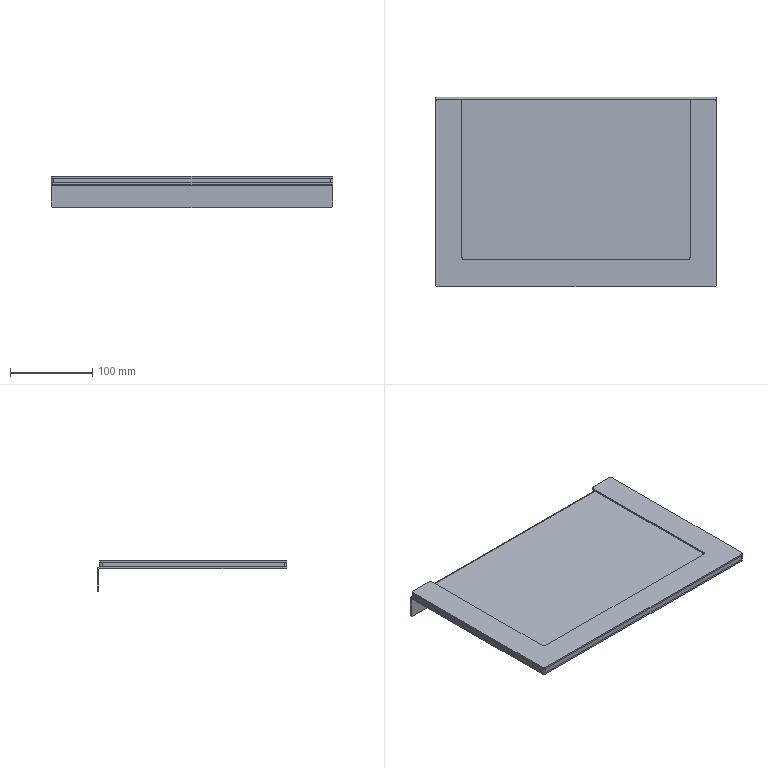Part | SolidWorks | features Fillet 4, ICE 2, EdgeFlange 1, FlatPattern 1, SMBaseFlange 1, SheetMetal 1 | 3 solids | 54 faces | box 342 x 230 x 38 mm | volume 314217 mm3 | plane 32 | cylinder 22 | commonest cylinder face diameters 6 x20 1.473 x1 5.473 x1
STEP:
#1=CARTESIAN_POINT('',(-171.,0.,-12.));
#2=VERTEX_POINT('',#1);
#3=CARTESIAN_POINT('',(-171.,0.,12.263));
#4=VERTEX_POINT('',#3);
#5=CARTESIAN_POINT('',(-171.,0.,15.));
#6=DIRECTION('',(0.,0.,1.));
#7=VECTOR('',#6,1000.);
#8=LINE('',#5,#7);
#9=EDGE_CURVE('',#2,#4,#8,.T.);
#10=ORIENTED_EDGE('',*,*,#9,.F.);
#11=CARTESIAN_POINT('',(-171.,-2.,-12.));
#12=VERTEX_POINT('',#11);
#13=CARTESIAN_POINT('',(-171.,-2.,-12.));
#14=DIRECTION('',(0.,-1.,0.));
#15=VECTOR('',#14,1000.);
#16=LINE('',#13,#15);
#17=EDGE_CURVE('',#2,#12,#16,.T.);
#18=ORIENTED_EDGE('',*,*,#17,.T.);
#19=CARTESIAN_POINT('',(-171.,-2.,12.263));
#20=VERTEX_POINT('',#19);
#21=CARTESIAN_POINT('',(-171.,-2.,15.));
#22=DIRECTION('',(0.,0.,1.));
#23=VECTOR('',#22,1000.);
#24=LINE('',#21,#23);
#25=EDGE_CURVE('',#12,#20,#24,.T.);
#26=ORIENTED_EDGE('',*,*,#25,.T.);
#27=CARTESIAN_POINT('',(-171.,-2.,12.263));
#28=DIRECTION('',(0.,1.,0.));
#29=VECTOR('',#28,1000.);
#30=LINE('',#27,#29);
#31=EDGE_CURVE('',#20,#4,#30,.T.);
#32=ORIENTED_EDGE('',*,*,#31,.T.);
#33=EDGE_LOOP('',(#10,#18,#26,#32));
#34=FACE_OUTER_BOUND('',#33,.T.);
#35=CARTESIAN_POINT('',(-171.,-2.,15.));
#36=DIRECTION('',(-1.,0.,0.));
#37=DIRECTION('',(0.,0.,1.));
#38=AXIS2_PLACEMENT_3D('',#35,#36,#37);
#39=PLANE('',#38);
#40=ADVANCED_FACE('',(#34),#39,.T.);
#41=CARTESIAN_POINT('',(168.,-2.,-15.));
#42=VERTEX_POINT('',#41);
#43=CARTESIAN_POINT('',(-168.,-2.,-15.));
#44=VERTEX_POINT('',#43);
#45=CARTESIAN_POINT('',(-171.,-2.,-15.));
#46=DIRECTION('',(-1.,0.,0.));
#47=VECTOR('',#46,1000.);
#48=LINE('',#45,#47);
#49=EDGE_CURVE('',#42,#44,#48,.T.);
#50=ORIENTED_EDGE('',*,*,#49,.F.);
#51=CARTESIAN_POINT('',(171.,-2.,-12.));
#52=VERTEX_POINT('',#51);
#53=CARTESIAN_POINT('',(168.,-2.,-12.));
#54=DIRECTION('',(0.,-1.,0.));
#55=DIRECTION('',(0.,0.,-1.));
#56=AXIS2_PLACEMENT_3D('',#53,#54,#55);
#57=CIRCLE('',#56,3.);
#58=EDGE_CURVE('',#42,#52,#57,.T.);
#59=ORIENTED_EDGE('',*,*,#58,.T.);
#60=CARTESIAN_POINT('',(171.,-2.,12.263));
#61=VERTEX_POINT('',#60);
#62=CARTESIAN_POINT('',(171.,-2.,15.));
#63=DIRECTION('',(0.,0.,-1.));
#64=VECTOR('',#63,1000.);
#65=LINE('',#62,#64);
#66=EDGE_CURVE('',#61,#52,#65,.T.);
#67=ORIENTED_EDGE('',*,*,#66,.F.);
#68=CARTESIAN_POINT('',(-171.,-2.,12.263));
#69=DIRECTION('',(1.,0.,0.));
#70=VECTOR('',#69,1000.);
#71=LINE('',#68,#70);
#72=EDGE_CURVE('',#20,#61,#71,.T.);
#73=ORIENTED_EDGE('',*,*,#72,.F.);
#74=ORIENTED_EDGE('',*,*,#25,.F.);
#75=CARTESIAN_POINT('',(-168.,-2.,-12.));
#76=DIRECTION('',(0.,-1.,0.));
#77=DIRECTION('',(0.,0.,-1.));
#78=AXIS2_PLACEMENT_3D('',#75,#76,#77);
#79=CIRCLE('',#78,3.);
#80=EDGE_CURVE('',#12,#44,#79,.T.);
#81=ORIENTED_EDGE('',*,*,#80,.T.);
#82=EDGE_LOOP('',(#50,#59,#67,#73,#74,#81));
#83=FACE_OUTER_BOUND('',#82,.T.);
#84=CARTESIAN_POINT('',(0.,-2.,0.));
#85=DIRECTION('',(0.,-1.,0.));
#86=DIRECTION('',(0.,0.,-1.));
#87=AXIS2_PLACEMENT_3D('',#84,#85,#86);
#88=PLANE('',#87);
#89=ADVANCED_FACE('',(#83),#88,.T.);
#90=CARTESIAN_POINT('',(171.,0.,12.263));
#91=VERTEX_POINT('',#90);
#92=CARTESIAN_POINT('',(171.,0.,-12.));
#93=VERTEX_POINT('',#92);
#94=CARTESIAN_POINT('',(171.,0.,15.));
#95=DIRECTION('',(0.,0.,-1.));
#96=VECTOR('',#95,1000.);
#97=LINE('',#94,#96);
#98=EDGE_CURVE('',#91,#93,#97,.T.);
#99=ORIENTED_EDGE('',*,*,#98,.T.);
#100=CARTESIAN_POINT('',(168.,0.,-15.));
#101=VERTEX_POINT('',#100);
#102=CARTESIAN_POINT('',(168.,0.,-12.));
#103=DIRECTION('',(0.,1.,0.));
#104=DIRECTION('',(0.,0.,-1.));
#105=AXIS2_PLACEMENT_3D('',#102,#103,#104);
#106=CIRCLE('',#105,3.);
#107=EDGE_CURVE('',#93,#101,#106,.T.);
#108=ORIENTED_EDGE('',*,*,#107,.T.);
#109=CARTESIAN_POINT('',(-168.,0.,-15.));
#110=VERTEX_POINT('',#109);
#111=CARTESIAN_POINT('',(-171.,0.,-15.));
#112=DIRECTION('',(-1.,0.,0.));
#113=VECTOR('',#112,1000.);
#114=LINE('',#111,#113);
#115=EDGE_CURVE('',#101,#110,#114,.T.);
#116=ORIENTED_EDGE('',*,*,#115,.T.);
#117=CARTESIAN_POINT('',(-168.,0.,-12.));
#118=DIRECTION('',(0.,1.,0.));
#119=DIRECTION('',(0.,0.,-1.));
#120=AXIS2_PLACEMENT_3D('',#117,#118,#119);
#121=CIRCLE('',#120,3.);
#122=EDGE_CURVE('',#110,#2,#121,.T.);
#123=ORIENTED_EDGE('',*,*,#122,.T.);
#124=ORIENTED_EDGE('',*,*,#9,.T.);
#125=CARTESIAN_POINT('',(-171.,0.,12.263));
#126=DIRECTION('',(1.,0.,0.));
#127=VECTOR('',#126,1000.);
#128=LINE('',#125,#127);
#129=EDGE_CURVE('',#4,#91,#128,.T.);
#130=ORIENTED_EDGE('',*,*,#129,.T.);
#131=EDGE_LOOP('',(#99,#108,#116,#123,#124,#130));
#132=FACE_OUTER_BOUND('',#131,.T.);
#133=CARTESIAN_POINT('',(0.,0.,0.));
#134=DIRECTION('',(0.,-1.,0.));
#135=DIRECTION('',(0.,0.,-1.));
#136=AXIS2_PLACEMENT_3D('',#133,#134,#135);
#137=PLANE('',#136);
#138=ADVANCED_FACE('',(#132),#137,.F.);
#139=ORIENTED_EDGE('',*,*,#66,.T.);
#140=CARTESIAN_POINT('',(171.,-2.,-12.));
#141=DIRECTION('',(0.,1.,0.));
#142=VECTOR('',#141,1000.);
#143=LINE('',#140,#142);
#144=EDGE_CURVE('',#52,#93,#143,.T.);
#145=ORIENTED_EDGE('',*,*,#144,.T.);
#146=ORIENTED_EDGE('',*,*,#98,.F.);
#147=CARTESIAN_POINT('',(171.,-2.,12.263));
#148=DIRECTION('',(0.,1.,0.));
#149=VECTOR('',#148,1000.);
#150=LINE('',#147,#149);
#151=EDGE_CURVE('',#61,#91,#150,.T.);
#152=ORIENTED_EDGE('',*,*,#151,.F.);
#153=EDGE_LOOP('',(#139,#145,#146,#152));
#154=FACE_OUTER_BOUND('',#153,.T.);
#155=CARTESIAN_POINT('',(171.,-2.,15.));
#156=DIRECTION('',(1.,0.,0.));
#157=DIRECTION('',(0.,0.,-1.));
#158=AXIS2_PLACEMENT_3D('',#155,#156,#157);
#159=PLANE('',#158);
#160=ADVANCED_FACE('',(#154),#159,.T.);
#161=ORIENTED_EDGE('',*,*,#115,.F.);
#162=CARTESIAN_POINT('',(168.,-2.,-15.));
#163=DIRECTION('',(0.,-1.,0.));
#164=VECTOR('',#163,1000.);
#165=LINE('',#162,#164);
#166=EDGE_CURVE('',#101,#42,#165,.T.);
#167=ORIENTED_EDGE('',*,*,#166,.T.);
#168=ORIENTED_EDGE('',*,*,#49,.T.);
#169=CARTESIAN_POINT('',(-168.,-2.,-15.));
#170=DIRECTION('',(0.,1.,0.));
#171=VECTOR('',#170,1000.);
#172=LINE('',#169,#171);
#173=EDGE_CURVE('',#44,#110,#172,.T.);
#174=ORIENTED_EDGE('',*,*,#173,.T.);
#175=EDGE_LOOP('',(#161,#167,#168,#174));
#176=FACE_OUTER_BOUND('',#175,.T.);
#177=CARTESIAN_POINT('',(-171.,-2.,-15.));
#178=DIRECTION('',(0.,0.,-1.));
#179=DIRECTION('',(-1.,0.,0.));
#180=AXIS2_PLACEMENT_3D('',#177,#178,#179);
#181=PLANE('',#180);
#182=ADVANCED_FACE('',(#176),#181,.T.);
#183=CARTESIAN_POINT('',(171.,-2.737,13.));
#184=VERTEX_POINT('',#183);
#185=CARTESIAN_POINT('',(171.,-2.737,15.));
#186=VERTEX_POINT('',#185);
#187=CARTESIAN_POINT('',(171.,-2.737,15.));
#188=DIRECTION('',(0.,0.,1.));
#189=VECTOR('',#188,1000.);
#190=LINE('',#187,#189);
#191=EDGE_CURVE('',#184,#186,#190,.T.);
#192=ORIENTED_EDGE('',*,*,#191,.F.);
#193=CARTESIAN_POINT('',(171.,-2.737,12.263));
#194=DIRECTION('',(1.,0.,0.));
#195=DIRECTION('',(0.,0.,1.));
#196=AXIS2_PLACEMENT_3D('',#193,#194,#195);
#197=CIRCLE('',#196,0.7366);
#198=EDGE_CURVE('',#61,#184,#197,.T.);
#199=ORIENTED_EDGE('',*,*,#198,.F.);
#200=ORIENTED_EDGE('',*,*,#151,.T.);
#201=CARTESIAN_POINT('',(171.,-2.737,12.263));
#202=DIRECTION('',(1.,0.,0.));
#203=DIRECTION('',(0.,0.,1.));
#204=AXIS2_PLACEMENT_3D('',#201,#202,#203);
#205=CIRCLE('',#204,2.737);
#206=EDGE_CURVE('',#91,#186,#205,.T.);
#207=ORIENTED_EDGE('',*,*,#206,.T.);
#208=EDGE_LOOP('',(#192,#199,#200,#207));
#209=FACE_OUTER_BOUND('',#208,.T.);
#210=CARTESIAN_POINT('',(171.,-2.737,12.263));
#211=DIRECTION('',(1.,0.,0.));
#212=DIRECTION('',(0.,0.,-1.));
#213=AXIS2_PLACEMENT_3D('',#210,#211,#212);
#214=PLANE('',#213);
#215=ADVANCED_FACE('',(#209),#214,.T.);
#216=CARTESIAN_POINT('',(-171.,-2.737,13.));
#217=VERTEX_POINT('',#216);
#218=CARTESIAN_POINT('',(-171.,-2.737,12.263));
#219=DIRECTION('',(-1.,0.,0.));
#220=DIRECTION('',(0.,0.,1.));
#221=AXIS2_PLACEMENT_3D('',#218,#219,#220);
#222=CIRCLE('',#221,0.7366);
#223=EDGE_CURVE('',#217,#20,#222,.T.);
#224=ORIENTED_EDGE('',*,*,#223,.F.);
#225=CARTESIAN_POINT('',(-171.,-2.737,15.));
#226=VERTEX_POINT('',#225);
#227=CARTESIAN_POINT('',(-171.,-2.737,13.));
#228=DIRECTION('',(0.,0.,1.));
#229=VECTOR('',#228,1000.);
#230=LINE('',#227,#229);
#231=EDGE_CURVE('',#217,#226,#230,.T.);
#232=ORIENTED_EDGE('',*,*,#231,.T.);
#233=CARTESIAN_POINT('',(-171.,-2.737,12.263));
#234=DIRECTION('',(-1.,0.,0.));
#235=DIRECTION('',(0.,0.,1.));
#236=AXIS2_PLACEMENT_3D('',#233,#234,#235);
#237=CIRCLE('',#236,2.737);
#238=EDGE_CURVE('',#226,#4,#237,.T.);
#239=ORIENTED_EDGE('',*,*,#238,.T.);
#240=ORIENTED_EDGE('',*,*,#31,.F.);
#241=EDGE_LOOP('',(#224,#232,#239,#240));
#242=FACE_OUTER_BOUND('',#241,.T.);
#243=CARTESIAN_POINT('',(-171.,-2.737,12.263));
#244=DIRECTION('',(1.,0.,0.));
#245=DIRECTION('',(0.,0.,-1.));
#246=AXIS2_PLACEMENT_3D('',#243,#244,#245);
#247=PLANE('',#246);
#248=ADVANCED_FACE('',(#242),#247,.F.);
#249=ORIENTED_EDGE('',*,*,#129,.F.);
#250=ORIENTED_EDGE('',*,*,#238,.F.);
#251=CARTESIAN_POINT('',(0.,-2.737,15.));
#252=DIRECTION('',(-1.,0.,0.));
#253=VECTOR('',#252,1000.);
#254=LINE('',#251,#253);
#255=EDGE_CURVE('',#186,#226,#254,.T.);
#256=ORIENTED_EDGE('',*,*,#255,.F.);
#257=ORIENTED_EDGE('',*,*,#206,.F.);
#258=EDGE_LOOP('',(#249,#250,#256,#257));
#259=FACE_OUTER_BOUND('',#258,.T.);
#260=CARTESIAN_POINT('',(-171.,-2.737,12.263));
#261=DIRECTION('',(-1.,0.,0.));
#262=DIRECTION('',(0.,0.,1.));
#263=AXIS2_PLACEMENT_3D('',#260,#261,#262);
#264=CYLINDRICAL_SURFACE('',#263,2.737);
#265=ADVANCED_FACE('',(#259),#264,.T.);
#266=ORIENTED_EDGE('',*,*,#72,.T.);
#267=ORIENTED_EDGE('',*,*,#198,.T.);
#268=CARTESIAN_POINT('',(171.,-2.737,13.));
#269=DIRECTION('',(-1.,0.,0.));
#270=VECTOR('',#269,1000.);
#271=LINE('',#268,#270);
#272=EDGE_CURVE('',#184,#217,#271,.T.);
#273=ORIENTED_EDGE('',*,*,#272,.T.);
#274=ORIENTED_EDGE('',*,*,#223,.T.);
#275=EDGE_LOOP('',(#266,#267,#273,#274));
#276=FACE_OUTER_BOUND('',#275,.T.);
#277=CARTESIAN_POINT('',(-171.,-2.737,12.263));
#278=DIRECTION('',(-1.,0.,0.));
#279=DIRECTION('',(0.,0.,1.));
#280=AXIS2_PLACEMENT_3D('',#277,#278,#279);
#281=CYLINDRICAL_SURFACE('',#280,0.7366);
#282=ADVANCED_FACE('',(#276),#281,.F.);
#283=CARTESIAN_POINT('',(-171.,-227.,13.));
#284=VERTEX_POINT('',#283);
#285=CARTESIAN_POINT('',(-171.,0.,13.));
#286=DIRECTION('',(0.,1.,0.));
#287=VECTOR('',#286,1000.);
#288=LINE('',#285,#287);
#289=EDGE_CURVE('',#284,#217,#288,.T.);
#290=ORIENTED_EDGE('',*,*,#289,.F.);
#291=CARTESIAN_POINT('',(-171.,-227.,15.));
#292=VERTEX_POINT('',#291);
#293=CARTESIAN_POINT('',(-171.,-227.,15.));
#294=DIRECTION('',(0.,0.,1.));
#295=VECTOR('',#294,1000.);
#296=LINE('',#293,#295);
#297=EDGE_CURVE('',#284,#292,#296,.T.);
#298=ORIENTED_EDGE('',*,*,#297,.T.);
#299=CARTESIAN_POINT('',(-171.,-2.,15.));
#300=DIRECTION('',(0.,1.,0.));
#301=VECTOR('',#300,1000.);
#302=LINE('',#299,#301);
#303=EDGE_CURVE('',#292,#226,#302,.T.);
#304=ORIENTED_EDGE('',*,*,#303,.T.);
#305=ORIENTED_EDGE('',*,*,#231,.F.);
#306=EDGE_LOOP('',(#290,#298,#304,#305));
#307=FACE_OUTER_BOUND('',#306,.T.);
#308=CARTESIAN_POINT('',(-171.,-2.,15.));
#309=DIRECTION('',(-1.,0.,0.));
#310=DIRECTION('',(0.,0.,1.));
#311=AXIS2_PLACEMENT_3D('',#308,#309,#310);
#312=PLANE('',#311);
#313=ADVANCED_FACE('',(#307),#312,.T.);
#314=CARTESIAN_POINT('',(171.,-227.,15.));
#315=VERTEX_POINT('',#314);
#316=CARTESIAN_POINT('',(171.,-230.,15.));
#317=DIRECTION('',(0.,-1.,0.));
#318=VECTOR('',#317,1000.);
#319=LINE('',#316,#318);
#320=EDGE_CURVE('',#186,#315,#319,.T.);
#321=ORIENTED_EDGE('',*,*,#320,.T.);
#322=CARTESIAN_POINT('',(171.,-227.,13.));
#323=VERTEX_POINT('',#322);
#324=CARTESIAN_POINT('',(171.,-227.,15.));
#325=DIRECTION('',(0.,0.,-1.));
#326=VECTOR('',#325,1000.);
#327=LINE('',#324,#326);
#328=EDGE_CURVE('',#315,#323,#327,.T.);
#329=ORIENTED_EDGE('',*,*,#328,.T.);
#330=CARTESIAN_POINT('',(171.,0.,13.));
#331=DIRECTION('',(0.,-1.,0.));
#332=VECTOR('',#331,1000.);
#333=LINE('',#330,#332);
#334=EDGE_CURVE('',#184,#323,#333,.T.);
#335=ORIENTED_EDGE('',*,*,#334,.F.);
#336=ORIENTED_EDGE('',*,*,#191,.T.);
#337=EDGE_LOOP('',(#321,#329,#335,#336));
#338=FACE_OUTER_BOUND('',#337,.T.);
#339=CARTESIAN_POINT('',(171.,-230.,15.));
#340=DIRECTION('',(1.,0.,0.));
#341=DIRECTION('',(0.,0.,-1.));
#342=AXIS2_PLACEMENT_3D('',#339,#340,#341);
#343=PLANE('',#342);
#344=ADVANCED_FACE('',(#338),#343,.T.);
#345=ORIENTED_EDGE('',*,*,#303,.F.);
#346=CARTESIAN_POINT('',(-168.,-230.,15.));
#347=VERTEX_POINT('',#346);
#348=CARTESIAN_POINT('',(-168.,-227.,15.));
#349=DIRECTION('',(0.,0.,1.));
#350=DIRECTION('',(0.,-1.,0.));
#351=AXIS2_PLACEMENT_3D('',#348,#349,#350);
#352=CIRCLE('',#351,3.);
#353=EDGE_CURVE('',#292,#347,#352,.T.);
#354=ORIENTED_EDGE('',*,*,#353,.T.);
#355=CARTESIAN_POINT('',(168.,-230.,15.));
#356=VERTEX_POINT('',#355);
#357=CARTESIAN_POINT('',(-171.,-230.,15.));
#358=DIRECTION('',(-1.,0.,0.));
#359=VECTOR('',#358,1000.);
#360=LINE('',#357,#359);
#361=EDGE_CURVE('',#356,#347,#360,.T.);
#362=ORIENTED_EDGE('',*,*,#361,.F.);
#363=CARTESIAN_POINT('',(168.,-227.,15.));
#364=DIRECTION('',(0.,0.,1.));
#365=DIRECTION('',(0.,-1.,0.));
#366=AXIS2_PLACEMENT_3D('',#363,#364,#365);
#367=CIRCLE('',#366,3.);
#368=EDGE_CURVE('',#356,#315,#367,.T.);
#369=ORIENTED_EDGE('',*,*,#368,.T.);
#370=ORIENTED_EDGE('',*,*,#320,.F.);
#371=ORIENTED_EDGE('',*,*,#255,.T.);
#372=EDGE_LOOP('',(#345,#354,#362,#369,#370,#371));
#373=FACE_OUTER_BOUND('',#372,.T.);
#374=CARTESIAN_POINT('',(0.,0.,15.));
#375=DIRECTION('',(0.,0.,1.));
#376=DIRECTION('',(0.,-1.,0.));
#377=AXIS2_PLACEMENT_3D('',#374,#375,#376);
#378=PLANE('',#377);
#379=ADVANCED_FACE('',(#373),#378,.T.);
#380=CARTESIAN_POINT('',(168.,-230.,13.));
#381=VERTEX_POINT('',#380);
#382=CARTESIAN_POINT('',(-168.,-230.,13.));
#383=VERTEX_POINT('',#382);
#384=CARTESIAN_POINT('',(0.,-230.,13.));
#385=DIRECTION('',(-1.,0.,0.));
#386=VECTOR('',#385,1000.);
#387=LINE('',#384,#386);
#388=EDGE_CURVE('',#381,#383,#387,.T.);
#389=ORIENTED_EDGE('',*,*,#388,.T.);
#390=CARTESIAN_POINT('',(-168.,-227.,13.));
#391=DIRECTION('',(0.,0.,-1.));
#392=DIRECTION('',(0.,-1.,0.));
#393=AXIS2_PLACEMENT_3D('',#390,#391,#392);
#394=CIRCLE('',#393,3.);
#395=EDGE_CURVE('',#383,#284,#394,.T.);
#396=ORIENTED_EDGE('',*,*,#395,.T.);
#397=ORIENTED_EDGE('',*,*,#289,.T.);
#398=ORIENTED_EDGE('',*,*,#272,.F.);
#399=ORIENTED_EDGE('',*,*,#334,.T.);
#400=CARTESIAN_POINT('',(168.,-227.,13.));
#401=DIRECTION('',(0.,0.,-1.));
#402=DIRECTION('',(0.,-1.,0.));
#403=AXIS2_PLACEMENT_3D('',#400,#401,#402);
#404=CIRCLE('',#403,3.);
#405=EDGE_CURVE('',#323,#381,#404,.T.);
#406=ORIENTED_EDGE('',*,*,#405,.T.);
#407=EDGE_LOOP('',(#389,#396,#397,#398,#399,#406));
#408=FACE_OUTER_BOUND('',#407,.T.);
#409=CARTESIAN_POINT('',(0.,0.,13.));
#410=DIRECTION('',(0.,0.,1.));
#411=DIRECTION('',(0.,-1.,0.));
#412=AXIS2_PLACEMENT_3D('',#409,#410,#411);
#413=PLANE('',#412);
#414=ADVANCED_FACE('',(#408),#413,.F.);
#415=ORIENTED_EDGE('',*,*,#361,.T.);
#416=CARTESIAN_POINT('',(-168.,-230.,15.));
#417=DIRECTION('',(0.,0.,-1.));
#418=VECTOR('',#417,1000.);
#419=LINE('',#416,#418);
#420=EDGE_CURVE('',#347,#383,#419,.T.);
#421=ORIENTED_EDGE('',*,*,#420,.T.);
#422=ORIENTED_EDGE('',*,*,#388,.F.);
#423=CARTESIAN_POINT('',(168.,-230.,15.));
#424=DIRECTION('',(0.,0.,1.));
#425=VECTOR('',#424,1000.);
#426=LINE('',#423,#425);
#427=EDGE_CURVE('',#381,#356,#426,.T.);
#428=ORIENTED_EDGE('',*,*,#427,.T.);
#429=EDGE_LOOP('',(#415,#421,#422,#428));
#430=FACE_OUTER_BOUND('',#429,.T.);
#431=CARTESIAN_POINT('',(-171.,-230.,15.));
#432=DIRECTION('',(0.,-1.,0.));
#433=DIRECTION('',(0.,0.,-1.));
#434=AXIS2_PLACEMENT_3D('',#431,#432,#433);
#435=PLANE('',#434);
#436=ADVANCED_FACE('',(#430),#435,.T.);
#437=ORIENTED_EDGE('',*,*,#58,.F.);
#438=ORIENTED_EDGE('',*,*,#166,.F.);
#439=ORIENTED_EDGE('',*,*,#107,.F.);
#440=ORIENTED_EDGE('',*,*,#144,.F.);
#441=EDGE_LOOP('',(#437,#438,#439,#440));
#442=FACE_OUTER_BOUND('',#441,.T.);
#443=CARTESIAN_POINT('',(168.,-2.,-12.));
#444=DIRECTION('',(0.,1.,0.));
#445=DIRECTION('',(0.,0.,1.));
#446=AXIS2_PLACEMENT_3D('',#443,#444,#445);
#447=CYLINDRICAL_SURFACE('',#446,3.);
#448=ADVANCED_FACE('',(#442),#447,.T.);
#449=ORIENTED_EDGE('',*,*,#80,.F.);
#450=ORIENTED_EDGE('',*,*,#17,.F.);
#451=ORIENTED_EDGE('',*,*,#122,.F.);
#452=ORIENTED_EDGE('',*,*,#173,.F.);
#453=EDGE_LOOP('',(#449,#450,#451,#452));
#454=FACE_OUTER_BOUND('',#453,.T.);
#455=CARTESIAN_POINT('',(-168.,-2.,-12.));
#456=DIRECTION('',(0.,1.,0.));
#457=DIRECTION('',(0.,0.,1.));
#458=AXIS2_PLACEMENT_3D('',#455,#456,#457);
#459=CYLINDRICAL_SURFACE('',#458,3.);
#460=ADVANCED_FACE('',(#454),#459,.T.);
#461=ORIENTED_EDGE('',*,*,#353,.F.);
#462=ORIENTED_EDGE('',*,*,#297,.F.);
#463=ORIENTED_EDGE('',*,*,#395,.F.);
#464=ORIENTED_EDGE('',*,*,#420,.F.);
#465=EDGE_LOOP('',(#461,#462,#463,#464));
#466=FACE_OUTER_BOUND('',#465,.T.);
#467=CARTESIAN_POINT('',(-168.,-227.,15.));
#468=DIRECTION('',(0.,0.,-1.));
#469=DIRECTION('',(0.,1.,0.));
#470=AXIS2_PLACEMENT_3D('',#467,#468,#469);
#471=CYLINDRICAL_SURFACE('',#470,3.);
#472=ADVANCED_FACE('',(#466),#471,.T.);
#473=ORIENTED_EDGE('',*,*,#368,.F.);
#474=ORIENTED_EDGE('',*,*,#427,.F.);
#475=ORIENTED_EDGE('',*,*,#405,.F.);
#476=ORIENTED_EDGE('',*,*,#328,.F.);
#477=EDGE_LOOP('',(#473,#474,#475,#476));
#478=FACE_OUTER_BOUND('',#477,.T.);
#479=CARTESIAN_POINT('',(168.,-227.,15.));
#480=DIRECTION('',(0.,0.,-1.));
#481=DIRECTION('',(0.,1.,0.));
#482=AXIS2_PLACEMENT_3D('',#479,#480,#481);
#483=CYLINDRICAL_SURFACE('',#482,3.);
#484=ADVANCED_FACE('',(#478),#483,.T.);
#485=CLOSED_SHELL('',(#40,#89,#138,#160,#182,#215,#248,#265,#282,#313,#344,#379,#414,#436,#448,#460,#472,#484));
#486=MANIFOLD_SOLID_BREP('',#485);
#487=CARTESIAN_POINT('',(-171.,-5.737,21.));
#488=VERTEX_POINT('',#487);
#489=CARTESIAN_POINT('',(-171.,-227.,21.));
#490=VERTEX_POINT('',#489);
#491=CARTESIAN_POINT('',(-171.,-230.,21.));
#492=DIRECTION('',(0.,-1.,0.));
#493=VECTOR('',#492,1000.);
#494=LINE('',#491,#493);
#495=EDGE_CURVE('',#488,#490,#494,.T.);
#496=ORIENTED_EDGE('',*,*,#495,.F.);
#497=CARTESIAN_POINT('',(-171.,-5.737,15.));
#498=VERTEX_POINT('',#497);
#499=CARTESIAN_POINT('',(-171.,-5.737,21.));
#500=DIRECTION('',(0.,0.,-1.));
#501=VECTOR('',#500,1000.);
#502=LINE('',#499,#501);
#503=EDGE_CURVE('',#488,#498,#502,.T.);
#504=ORIENTED_EDGE('',*,*,#503,.T.);
#505=CARTESIAN_POINT('',(-171.,-227.,15.));
#506=VERTEX_POINT('',#505);
#507=CARTESIAN_POINT('',(-171.,-230.,15.));
#508=DIRECTION('',(0.,-1.,0.));
#509=VECTOR('',#508,1000.);
#510=LINE('',#507,#509);
#511=EDGE_CURVE('',#498,#506,#510,.T.);
#512=ORIENTED_EDGE('',*,*,#511,.T.);
#513=CARTESIAN_POINT('',(-171.,-227.,21.));
#514=DIRECTION('',(0.,0.,1.));
#515=VECTOR('',#514,1000.);
#516=LINE('',#513,#515);
#517=EDGE_CURVE('',#506,#490,#516,.T.);
#518=ORIENTED_EDGE('',*,*,#517,.T.);
#519=EDGE_LOOP('',(#496,#504,#512,#518));
#520=FACE_OUTER_BOUND('',#519,.T.);
#521=CARTESIAN_POINT('',(-171.,-230.,21.));
#522=DIRECTION('',(1.,0.,0.));
#523=DIRECTION('',(0.,0.,-1.));
#524=AXIS2_PLACEMENT_3D('',#521,#522,#523);
#525=PLANE('',#524);
#526=ADVANCED_FACE('',(#520),#525,.F.);
#527=CARTESIAN_POINT('',(-168.,-230.,15.));
#528=VERTEX_POINT('',#527);
#529=CARTESIAN_POINT('',(168.,-230.,15.));
#530=VERTEX_POINT('',#529);
#531=CARTESIAN_POINT('',(171.,-230.,15.));
#532=DIRECTION('',(1.,0.,0.));
#533=VECTOR('',#532,1000.);
#534=LINE('',#531,#533);
#535=EDGE_CURVE('',#528,#530,#534,.T.);
#536=ORIENTED_EDGE('',*,*,#535,.T.);
#537=CARTESIAN_POINT('',(168.,-230.,21.));
#538=VERTEX_POINT('',#537);
#539=CARTESIAN_POINT('',(168.,-230.,21.));
#540=DIRECTION('',(0.,0.,1.));
#541=VECTOR('',#540,1000.);
#542=LINE('',#539,#541);
#543=EDGE_CURVE('',#530,#538,#542,.T.);
#544=ORIENTED_EDGE('',*,*,#543,.T.);
#545=CARTESIAN_POINT('',(-168.,-230.,21.));
#546=VERTEX_POINT('',#545);
#547=CARTESIAN_POINT('',(-171.,-230.,21.));
#548=DIRECTION('',(1.,0.,0.));
#549=VECTOR('',#548,1000.);
#550=LINE('',#547,#549);
#551=EDGE_CURVE('',#546,#538,#550,.T.);
#552=ORIENTED_EDGE('',*,*,#551,.F.);
#553=CARTESIAN_POINT('',(-168.,-230.,21.));
#554=DIRECTION('',(0.,0.,-1.));
#555=VECTOR('',#554,1000.);
#556=LINE('',#553,#555);
#557=EDGE_CURVE('',#546,#528,#556,.T.);
#558=ORIENTED_EDGE('',*,*,#557,.T.);
#559=EDGE_LOOP('',(#536,#544,#552,#558));
#560=FACE_OUTER_BOUND('',#559,.T.);
#561=CARTESIAN_POINT('',(171.,-230.,21.));
#562=DIRECTION('',(0.,1.,0.));
#563=DIRECTION('',(0.,0.,1.));
#564=AXIS2_PLACEMENT_3D('',#561,#562,#563);
#565=PLANE('',#564);
#566=ADVANCED_FACE('',(#560),#565,.F.);
#567=CARTESIAN_POINT('',(171.,-227.,21.));
#568=VERTEX_POINT('',#567);
#569=CARTESIAN_POINT('',(171.,-5.737,21.));
#570=VERTEX_POINT('',#569);
#571=CARTESIAN_POINT('',(171.,-230.,21.));
#572=DIRECTION('',(0.,1.,0.));
#573=VECTOR('',#572,1000.);
#574=LINE('',#571,#573);
#575=EDGE_CURVE('',#568,#570,#574,.T.);
#576=ORIENTED_EDGE('',*,*,#575,.F.);
#577=CARTESIAN_POINT('',(171.,-227.,15.));
#578=VERTEX_POINT('',#577);
#579=CARTESIAN_POINT('',(171.,-227.,21.));
#580=DIRECTION('',(0.,0.,-1.));
#581=VECTOR('',#580,1000.);
#582=LINE('',#579,#581);
#583=EDGE_CURVE('',#568,#578,#582,.T.);
#584=ORIENTED_EDGE('',*,*,#583,.T.);
#585=CARTESIAN_POINT('',(171.,-5.737,15.));
#586=VERTEX_POINT('',#585);
#587=CARTESIAN_POINT('',(171.,-230.,15.));
#588=DIRECTION('',(0.,1.,0.));
#589=VECTOR('',#588,1000.);
#590=LINE('',#587,#589);
#591=EDGE_CURVE('',#578,#586,#590,.T.);
#592=ORIENTED_EDGE('',*,*,#591,.T.);
#593=CARTESIAN_POINT('',(171.,-5.737,21.));
#594=DIRECTION('',(0.,0.,1.));
#595=VECTOR('',#594,1000.);
#596=LINE('',#593,#595);
#597=EDGE_CURVE('',#586,#570,#596,.T.);
#598=ORIENTED_EDGE('',*,*,#597,.T.);
#599=EDGE_LOOP('',(#576,#584,#592,#598));
#600=FACE_OUTER_BOUND('',#599,.T.);
#601=CARTESIAN_POINT('',(171.,-230.,21.));
#602=DIRECTION('',(-1.,0.,0.));
#603=DIRECTION('',(0.,0.,1.));
#604=AXIS2_PLACEMENT_3D('',#601,#602,#603);
#605=PLANE('',#604);
#606=ADVANCED_FACE('',(#600),#605,.F.);
#607=CARTESIAN_POINT('',(168.,-2.737,21.));
#608=VERTEX_POINT('',#607);
#609=CARTESIAN_POINT('',(154.,-2.737,21.));
#610=VERTEX_POINT('',#609);
#611=CARTESIAN_POINT('',(171.,-2.737,21.));
#612=DIRECTION('',(-1.,0.,0.));
#613=VECTOR('',#612,1000.);
#614=LINE('',#611,#613);
#615=EDGE_CURVE('',#608,#610,#614,.T.);
#616=ORIENTED_EDGE('',*,*,#615,.F.);
#617=CARTESIAN_POINT('',(168.,-2.737,15.));
#618=VERTEX_POINT('',#617);
#619=CARTESIAN_POINT('',(168.,-2.737,21.));
#620=DIRECTION('',(0.,0.,-1.));
#621=VECTOR('',#620,1000.);
#622=LINE('',#619,#621);
#623=EDGE_CURVE('',#608,#618,#622,.T.);
#624=ORIENTED_EDGE('',*,*,#623,.T.);
#625=CARTESIAN_POINT('',(154.,-2.737,15.));
#626=VERTEX_POINT('',#625);
#627=CARTESIAN_POINT('',(171.,-2.737,15.));
#628=DIRECTION('',(-1.,0.,0.));
#629=VECTOR('',#628,1000.);
#630=LINE('',#627,#629);
#631=EDGE_CURVE('',#618,#626,#630,.T.);
#632=ORIENTED_EDGE('',*,*,#631,.T.);
#633=CARTESIAN_POINT('',(154.,-2.737,21.));
#634=DIRECTION('',(0.,0.,1.));
#635=VECTOR('',#634,1000.);
#636=LINE('',#633,#635);
#637=EDGE_CURVE('',#626,#610,#636,.T.);
#638=ORIENTED_EDGE('',*,*,#637,.T.);
#639=EDGE_LOOP('',(#616,#624,#632,#638));
#640=FACE_OUTER_BOUND('',#639,.T.);
#641=CARTESIAN_POINT('',(171.,-2.737,21.));
#642=DIRECTION('',(0.,-1.,0.));
#643=DIRECTION('',(0.,0.,-1.));
#644=AXIS2_PLACEMENT_3D('',#641,#642,#643);
#645=PLANE('',#644);
#646=ADVANCED_FACE('',(#640),#645,.F.);
#647=CARTESIAN_POINT('',(151.,-5.737,15.));
#648=VERTEX_POINT('',#647);
#649=CARTESIAN_POINT('',(151.,-207.,15.));
#650=VERTEX_POINT('',#649);
#651=CARTESIAN_POINT('',(151.,-210.,15.));
#652=DIRECTION('',(0.,-1.,0.));
#653=VECTOR('',#652,1000.);
#654=LINE('',#651,#653);
#655=EDGE_CURVE('',#648,#650,#654,.T.);
#656=ORIENTED_EDGE('',*,*,#655,.T.);
#657=CARTESIAN_POINT('',(151.,-207.,21.));
#658=VERTEX_POINT('',#657);
#659=CARTESIAN_POINT('',(151.,-207.,21.));
#660=DIRECTION('',(0.,0.,1.));
#661=VECTOR('',#660,1000.);
#662=LINE('',#659,#661);
#663=EDGE_CURVE('',#650,#658,#662,.T.);
#664=ORIENTED_EDGE('',*,*,#663,.T.);
#665=CARTESIAN_POINT('',(151.,-5.737,21.));
#666=VERTEX_POINT('',#665);
#667=CARTESIAN_POINT('',(151.,-210.,21.));
#668=DIRECTION('',(0.,-1.,0.));
#669=VECTOR('',#668,1000.);
#670=LINE('',#667,#669);
#671=EDGE_CURVE('',#666,#658,#670,.T.);
#672=ORIENTED_EDGE('',*,*,#671,.F.);
#673=CARTESIAN_POINT('',(151.,-5.737,21.));
#674=DIRECTION('',(0.,0.,-1.));
#675=VECTOR('',#674,1000.);
#676=LINE('',#673,#675);
#677=EDGE_CURVE('',#666,#648,#676,.T.);
#678=ORIENTED_EDGE('',*,*,#677,.T.);
#679=EDGE_LOOP('',(#656,#664,#672,#678));
#680=FACE_OUTER_BOUND('',#679,.T.);
#681=CARTESIAN_POINT('',(151.,-210.,21.));
#682=DIRECTION('',(1.,0.,0.));
#683=DIRECTION('',(0.,0.,-1.));
#684=AXIS2_PLACEMENT_3D('',#681,#682,#683);
#685=PLANE('',#684);
#686=ADVANCED_FACE('',(#680),#685,.F.);
#687=CARTESIAN_POINT('',(148.,-210.,21.));
#688=VERTEX_POINT('',#687);
#689=CARTESIAN_POINT('',(-148.,-210.,21.));
#690=VERTEX_POINT('',#689);
#691=CARTESIAN_POINT('',(-151.,-210.,21.));
#692=DIRECTION('',(-1.,0.,0.));
#693=VECTOR('',#692,1000.);
#694=LINE('',#691,#693);
#695=EDGE_CURVE('',#688,#690,#694,.T.);
#696=ORIENTED_EDGE('',*,*,#695,.F.);
#697=CARTESIAN_POINT('',(148.,-210.,15.));
#698=VERTEX_POINT('',#697);
#699=CARTESIAN_POINT('',(148.,-210.,15.));
#700=DIRECTION('',(0.,0.,-1.));
#701=VECTOR('',#700,1000.);
#702=LINE('',#699,#701);
#703=EDGE_CURVE('',#688,#698,#702,.T.);
#704=ORIENTED_EDGE('',*,*,#703,.T.);
#705=CARTESIAN_POINT('',(-148.,-210.,15.));
#706=VERTEX_POINT('',#705);
#707=CARTESIAN_POINT('',(-151.,-210.,15.));
#708=DIRECTION('',(-1.,0.,0.));
#709=VECTOR('',#708,1000.);
#710=LINE('',#707,#709);
#711=EDGE_CURVE('',#698,#706,#710,.T.);
#712=ORIENTED_EDGE('',*,*,#711,.T.);
#713=CARTESIAN_POINT('',(-148.,-210.,21.));
#714=DIRECTION('',(0.,0.,1.));
#715=VECTOR('',#714,1000.);
#716=LINE('',#713,#715);
#717=EDGE_CURVE('',#706,#690,#716,.T.);
#718=ORIENTED_EDGE('',*,*,#717,.T.);
#719=EDGE_LOOP('',(#696,#704,#712,#718));
#720=FACE_OUTER_BOUND('',#719,.T.);
#721=CARTESIAN_POINT('',(-151.,-210.,21.));
#722=DIRECTION('',(0.,-1.,0.));
#723=DIRECTION('',(0.,0.,-1.));
#724=AXIS2_PLACEMENT_3D('',#721,#722,#723);
#725=PLANE('',#724);
#726=ADVANCED_FACE('',(#720),#725,.F.);
#727=CARTESIAN_POINT('',(-151.,-207.,21.));
#728=VERTEX_POINT('',#727);
#729=CARTESIAN_POINT('',(-151.,-5.737,21.));
#730=VERTEX_POINT('',#729);
#731=CARTESIAN_POINT('',(-151.,-210.,21.));
#732=DIRECTION('',(0.,1.,0.));
#733=VECTOR('',#732,1000.);
#734=LINE('',#731,#733);
#735=EDGE_CURVE('',#728,#730,#734,.T.);
#736=ORIENTED_EDGE('',*,*,#735,.F.);
#737=CARTESIAN_POINT('',(-151.,-207.,15.));
#738=VERTEX_POINT('',#737);
#739=CARTESIAN_POINT('',(-151.,-207.,15.));
#740=DIRECTION('',(0.,0.,-1.));
#741=VECTOR('',#740,1000.);
#742=LINE('',#739,#741);
#743=EDGE_CURVE('',#728,#738,#742,.T.);
#744=ORIENTED_EDGE('',*,*,#743,.T.);
#745=CARTESIAN_POINT('',(-151.,-5.737,15.));
#746=VERTEX_POINT('',#745);
#747=CARTESIAN_POINT('',(-151.,-210.,15.));
#748=DIRECTION('',(0.,1.,0.));
#749=VECTOR('',#748,1000.);
#750=LINE('',#747,#749);
#751=EDGE_CURVE('',#738,#746,#750,.T.);
#752=ORIENTED_EDGE('',*,*,#751,.T.);
#753=CARTESIAN_POINT('',(-151.,-5.737,21.));
#754=DIRECTION('',(0.,0.,1.));
#755=VECTOR('',#754,1000.);
#756=LINE('',#753,#755);
#757=EDGE_CURVE('',#746,#730,#756,.T.);
#758=ORIENTED_EDGE('',*,*,#757,.T.);
#759=EDGE_LOOP('',(#736,#744,#752,#758));
#760=FACE_OUTER_BOUND('',#759,.T.);
#761=CARTESIAN_POINT('',(-151.,-210.,21.));
#762=DIRECTION('',(-1.,0.,0.));
#763=DIRECTION('',(0.,-1.,0.));
#764=AXIS2_PLACEMENT_3D('',#761,#762,#763);
#765=PLANE('',#764);
#766=ADVANCED_FACE('',(#760),#765,.F.);
#767=CARTESIAN_POINT('',(-154.,-2.737,21.));
#768=VERTEX_POINT('',#767);
#769=CARTESIAN_POINT('',(-168.,-2.737,21.));
#770=VERTEX_POINT('',#769);
#771=CARTESIAN_POINT('',(-171.,-2.737,21.));
#772=DIRECTION('',(-1.,0.,0.));
#773=VECTOR('',#772,1000.);
#774=LINE('',#771,#773);
#775=EDGE_CURVE('',#768,#770,#774,.T.);
#776=ORIENTED_EDGE('',*,*,#775,.F.);
#777=CARTESIAN_POINT('',(-154.,-2.737,15.));
#778=VERTEX_POINT('',#777);
#779=CARTESIAN_POINT('',(-154.,-2.737,21.));
#780=DIRECTION('',(0.,0.,-1.));
#781=VECTOR('',#780,1000.);
#782=LINE('',#779,#781);
#783=EDGE_CURVE('',#768,#778,#782,.T.);
#784=ORIENTED_EDGE('',*,*,#783,.T.);
#785=CARTESIAN_POINT('',(-168.,-2.737,15.));
#786=VERTEX_POINT('',#785);
#787=CARTESIAN_POINT('',(-171.,-2.737,15.));
#788=DIRECTION('',(-1.,0.,0.));
#789=VECTOR('',#788,1000.);
#790=LINE('',#787,#789);
#791=EDGE_CURVE('',#778,#786,#790,.T.);
#792=ORIENTED_EDGE('',*,*,#791,.T.);
#793=CARTESIAN_POINT('',(-168.,-2.737,21.));
#794=DIRECTION('',(0.,0.,1.));
#795=VECTOR('',#794,1000.);
#796=LINE('',#793,#795);
#797=EDGE_CURVE('',#786,#770,#796,.T.);
#798=ORIENTED_EDGE('',*,*,#797,.T.);
#799=EDGE_LOOP('',(#776,#784,#792,#798));
#800=FACE_OUTER_BOUND('',#799,.T.);
#801=CARTESIAN_POINT('',(-171.,-2.737,21.));
#802=DIRECTION('',(0.,-1.,0.));
#803=DIRECTION('',(1.,0.,0.));
#804=AXIS2_PLACEMENT_3D('',#801,#802,#803);
#805=PLANE('',#804);
#806=ADVANCED_FACE('',(#800),#805,.F.);
#807=ORIENTED_EDGE('',*,*,#551,.T.);
#808=CARTESIAN_POINT('',(168.,-227.,21.));
#809=DIRECTION('',(0.,0.,1.));
#810=DIRECTION('',(-1.,0.,0.));
#811=AXIS2_PLACEMENT_3D('',#808,#809,#810);
#812=CIRCLE('',#811,3.);
#813=EDGE_CURVE('',#538,#568,#812,.T.);
#814=ORIENTED_EDGE('',*,*,#813,.T.);
#815=ORIENTED_EDGE('',*,*,#575,.T.);
#816=CARTESIAN_POINT('',(168.,-5.737,21.));
#817=DIRECTION('',(0.,0.,1.));
#818=DIRECTION('',(-1.,0.,0.));
#819=AXIS2_PLACEMENT_3D('',#816,#817,#818);
#820=CIRCLE('',#819,3.);
#821=EDGE_CURVE('',#570,#608,#820,.T.);
#822=ORIENTED_EDGE('',*,*,#821,.T.);
#823=ORIENTED_EDGE('',*,*,#615,.T.);
#824=CARTESIAN_POINT('',(154.,-5.737,21.));
#825=DIRECTION('',(0.,0.,1.));
#826=DIRECTION('',(-1.,0.,0.));
#827=AXIS2_PLACEMENT_3D('',#824,#825,#826);
#828=CIRCLE('',#827,3.);
#829=EDGE_CURVE('',#610,#666,#828,.T.);
#830=ORIENTED_EDGE('',*,*,#829,.T.);
#831=ORIENTED_EDGE('',*,*,#671,.T.);
#832=CARTESIAN_POINT('',(148.,-207.,21.));
#833=DIRECTION('',(0.,0.,-1.));
#834=DIRECTION('',(-1.,0.,0.));
#835=AXIS2_PLACEMENT_3D('',#832,#833,#834);
#836=CIRCLE('',#835,3.);
#837=EDGE_CURVE('',#658,#688,#836,.T.);
#838=ORIENTED_EDGE('',*,*,#837,.T.);
#839=ORIENTED_EDGE('',*,*,#695,.T.);
#840=CARTESIAN_POINT('',(-148.,-207.,21.));
#841=DIRECTION('',(0.,0.,-1.));
#842=DIRECTION('',(-1.,0.,0.));
#843=AXIS2_PLACEMENT_3D('',#840,#841,#842);
#844=CIRCLE('',#843,3.);
#845=EDGE_CURVE('',#690,#728,#844,.T.);
#846=ORIENTED_EDGE('',*,*,#845,.T.);
#847=ORIENTED_EDGE('',*,*,#735,.T.);
#848=CARTESIAN_POINT('',(-154.,-5.737,21.));
#849=DIRECTION('',(0.,0.,1.));
#850=DIRECTION('',(-1.,0.,0.));
#851=AXIS2_PLACEMENT_3D('',#848,#849,#850);
#852=CIRCLE('',#851,3.);
#853=EDGE_CURVE('',#730,#768,#852,.T.);
#854=ORIENTED_EDGE('',*,*,#853,.T.);
#855=ORIENTED_EDGE('',*,*,#775,.T.);
#856=CARTESIAN_POINT('',(-168.,-5.737,21.));
#857=DIRECTION('',(0.,0.,1.));
#858=DIRECTION('',(-1.,0.,0.));
#859=AXIS2_PLACEMENT_3D('',#856,#857,#858);
#860=CIRCLE('',#859,3.);
#861=EDGE_CURVE('',#770,#488,#860,.T.);
#862=ORIENTED_EDGE('',*,*,#861,.T.);
#863=ORIENTED_EDGE('',*,*,#495,.T.);
#864=CARTESIAN_POINT('',(-168.,-227.,21.));
#865=DIRECTION('',(0.,0.,1.));
#866=DIRECTION('',(-1.,0.,0.));
#867=AXIS2_PLACEMENT_3D('',#864,#865,#866);
#868=CIRCLE('',#867,3.);
#869=EDGE_CURVE('',#490,#546,#868,.T.);
#870=ORIENTED_EDGE('',*,*,#869,.T.);
#871=EDGE_LOOP('',(#807,#814,#815,#822,#823,#830,#831,#838,#839,#846,#847,#854,#855,#862,#863,#870));
#872=FACE_OUTER_BOUND('',#871,.T.);
#873=CARTESIAN_POINT('',(0.,0.,21.));
#874=DIRECTION('',(0.,0.,-1.));
#875=DIRECTION('',(-1.,0.,0.));
#876=AXIS2_PLACEMENT_3D('',#873,#874,#875);
#877=PLANE('',#876);
#878=ADVANCED_FACE('',(#872),#877,.F.);
#879=ORIENTED_EDGE('',*,*,#591,.F.);
#880=CARTESIAN_POINT('',(168.,-227.,15.));
#881=DIRECTION('',(0.,0.,-1.));
#882=DIRECTION('',(-1.,0.,0.));
#883=AXIS2_PLACEMENT_3D('',#880,#881,#882);
#884=CIRCLE('',#883,3.);
#885=EDGE_CURVE('',#578,#530,#884,.T.);
#886=ORIENTED_EDGE('',*,*,#885,.T.);
#887=ORIENTED_EDGE('',*,*,#535,.F.);
#888=CARTESIAN_POINT('',(-168.,-227.,15.));
#889=DIRECTION('',(0.,0.,-1.));
#890=DIRECTION('',(-1.,0.,0.));
#891=AXIS2_PLACEMENT_3D('',#888,#889,#890);
#892=CIRCLE('',#891,3.);
#893=EDGE_CURVE('',#528,#506,#892,.T.);
#894=ORIENTED_EDGE('',*,*,#893,.T.);
#895=ORIENTED_EDGE('',*,*,#511,.F.);
#896=CARTESIAN_POINT('',(-168.,-5.737,15.));
#897=DIRECTION('',(0.,0.,-1.));
#898=DIRECTION('',(-1.,0.,0.));
#899=AXIS2_PLACEMENT_3D('',#896,#897,#898);
#900=CIRCLE('',#899,3.);
#901=EDGE_CURVE('',#498,#786,#900,.T.);
#902=ORIENTED_EDGE('',*,*,#901,.T.);
#903=ORIENTED_EDGE('',*,*,#791,.F.);
#904=CARTESIAN_POINT('',(-154.,-5.737,15.));
#905=DIRECTION('',(0.,0.,-1.));
#906=DIRECTION('',(-1.,0.,0.));
#907=AXIS2_PLACEMENT_3D('',#904,#905,#906);
#908=CIRCLE('',#907,3.);
#909=EDGE_CURVE('',#778,#746,#908,.T.);
#910=ORIENTED_EDGE('',*,*,#909,.T.);
#911=ORIENTED_EDGE('',*,*,#751,.F.);
#912=CARTESIAN_POINT('',(-148.,-207.,15.));
#913=DIRECTION('',(0.,0.,1.));
#914=DIRECTION('',(-1.,0.,0.));
#915=AXIS2_PLACEMENT_3D('',#912,#913,#914);
#916=CIRCLE('',#915,3.);
#917=EDGE_CURVE('',#738,#706,#916,.T.);
#918=ORIENTED_EDGE('',*,*,#917,.T.);
#919=ORIENTED_EDGE('',*,*,#711,.F.);
#920=CARTESIAN_POINT('',(148.,-207.,15.));
#921=DIRECTION('',(0.,0.,1.));
#922=DIRECTION('',(-1.,0.,0.));
#923=AXIS2_PLACEMENT_3D('',#920,#921,#922);
#924=CIRCLE('',#923,3.);
#925=EDGE_CURVE('',#698,#650,#924,.T.);
#926=ORIENTED_EDGE('',*,*,#925,.T.);
#927=ORIENTED_EDGE('',*,*,#655,.F.);
#928=CARTESIAN_POINT('',(154.,-5.737,15.));
#929=DIRECTION('',(0.,0.,-1.));
#930=DIRECTION('',(-1.,0.,0.));
#931=AXIS2_PLACEMENT_3D('',#928,#929,#930);
#932=CIRCLE('',#931,3.);
#933=EDGE_CURVE('',#648,#626,#932,.T.);
#934=ORIENTED_EDGE('',*,*,#933,.T.);
#935=ORIENTED_EDGE('',*,*,#631,.F.);
#936=CARTESIAN_POINT('',(168.,-5.737,15.));
#937=DIRECTION('',(0.,0.,-1.));
#938=DIRECTION('',(-1.,0.,0.));
#939=AXIS2_PLACEMENT_3D('',#936,#937,#938);
#940=CIRCLE('',#939,3.);
#941=EDGE_CURVE('',#618,#586,#940,.T.);
#942=ORIENTED_EDGE('',*,*,#941,.T.);
#943=EDGE_LOOP('',(#879,#886,#887,#894,#895,#902,#903,#910,#911,#918,#919,#926,#927,#934,#935,#942));
#944=FACE_OUTER_BOUND('',#943,.T.);
#945=CARTESIAN_POINT('',(0.,0.,15.));
#946=DIRECTION('',(0.,0.,-1.));
#947=DIRECTION('',(-1.,0.,0.));
#948=AXIS2_PLACEMENT_3D('',#945,#946,#947);
#949=PLANE('',#948);
#950=ADVANCED_FACE('',(#944),#949,.T.);
#951=ORIENTED_EDGE('',*,*,#853,.F.);
#952=ORIENTED_EDGE('',*,*,#757,.F.);
#953=ORIENTED_EDGE('',*,*,#909,.F.);
#954=ORIENTED_EDGE('',*,*,#783,.F.);
#955=EDGE_LOOP('',(#951,#952,#953,#954));
#956=FACE_OUTER_BOUND('',#955,.T.);
#957=CARTESIAN_POINT('',(-154.,-5.737,21.));
#958=DIRECTION('',(0.,0.,-1.));
#959=DIRECTION('',(-1.,0.,0.));
#960=AXIS2_PLACEMENT_3D('',#957,#958,#959);
#961=CYLINDRICAL_SURFACE('',#960,3.);
#962=ADVANCED_FACE('',(#956),#961,.T.);
#963=ORIENTED_EDGE('',*,*,#861,.F.);
#964=ORIENTED_EDGE('',*,*,#797,.F.);
#965=ORIENTED_EDGE('',*,*,#901,.F.);
#966=ORIENTED_EDGE('',*,*,#503,.F.);
#967=EDGE_LOOP('',(#963,#964,#965,#966));
#968=FACE_OUTER_BOUND('',#967,.T.);
#969=CARTESIAN_POINT('',(-168.,-5.737,21.));
#970=DIRECTION('',(0.,0.,-1.));
#971=DIRECTION('',(-1.,0.,0.));
#972=AXIS2_PLACEMENT_3D('',#969,#970,#971);
#973=CYLINDRICAL_SURFACE('',#972,3.);
#974=ADVANCED_FACE('',(#968),#973,.T.);
#975=ORIENTED_EDGE('',*,*,#869,.F.);
#976=ORIENTED_EDGE('',*,*,#517,.F.);
#977=ORIENTED_EDGE('',*,*,#893,.F.);
#978=ORIENTED_EDGE('',*,*,#557,.F.);
#979=EDGE_LOOP('',(#975,#976,#977,#978));
#980=FACE_OUTER_BOUND('',#979,.T.);
#981=CARTESIAN_POINT('',(-168.,-227.,21.));
#982=DIRECTION('',(0.,0.,-1.));
#983=DIRECTION('',(-1.,0.,0.));
#984=AXIS2_PLACEMENT_3D('',#981,#982,#983);
#985=CYLINDRICAL_SURFACE('',#984,3.);
#986=ADVANCED_FACE('',(#980),#985,.T.);
#987=ORIENTED_EDGE('',*,*,#837,.F.);
#988=ORIENTED_EDGE('',*,*,#663,.F.);
#989=ORIENTED_EDGE('',*,*,#925,.F.);
#990=ORIENTED_EDGE('',*,*,#703,.F.);
#991=EDGE_LOOP('',(#987,#988,#989,#990));
#992=FACE_OUTER_BOUND('',#991,.T.);
#993=CARTESIAN_POINT('',(148.,-207.,21.));
#994=DIRECTION('',(0.,0.,1.));
#995=DIRECTION('',(1.,0.,0.));
#996=AXIS2_PLACEMENT_3D('',#993,#994,#995);
#997=CYLINDRICAL_SURFACE('',#996,3.);
#998=ADVANCED_FACE('',(#992),#997,.F.);
#999=ORIENTED_EDGE('',*,*,#845,.F.);
#1000=ORIENTED_EDGE('',*,*,#717,.F.);
#1001=ORIENTED_EDGE('',*,*,#917,.F.);
#1002=ORIENTED_EDGE('',*,*,#743,.F.);
#1003=EDGE_LOOP('',(#999,#1000,#1001,#1002));
#1004=FACE_OUTER_BOUND('',#1003,.T.);
#1005=CARTESIAN_POINT('',(-148.,-207.,21.));
#1006=DIRECTION('',(0.,0.,1.));
#1007=DIRECTION('',(1.,0.,0.));
#1008=AXIS2_PLACEMENT_3D('',#1005,#1006,#1007);
#1009=CYLINDRICAL_SURFACE('',#1008,3.);
#1010=ADVANCED_FACE('',(#1004),#1009,.F.);
#1011=ORIENTED_EDGE('',*,*,#813,.F.);
#1012=ORIENTED_EDGE('',*,*,#543,.F.);
#1013=ORIENTED_EDGE('',*,*,#885,.F.);
#1014=ORIENTED_EDGE('',*,*,#583,.F.);
#1015=EDGE_LOOP('',(#1011,#1012,#1013,#1014));
#1016=FACE_OUTER_BOUND('',#1015,.T.);
#1017=CARTESIAN_POINT('',(168.,-227.,21.));
#1018=DIRECTION('',(0.,0.,-1.));
#1019=DIRECTION('',(-1.,0.,0.));
#1020=AXIS2_PLACEMENT_3D('',#1017,#1018,#1019);
#1021=CYLINDRICAL_SURFACE('',#1020,3.);
#1022=ADVANCED_FACE('',(#1016),#1021,.T.);
#1023=ORIENTED_EDGE('',*,*,#821,.F.);
#1024=ORIENTED_EDGE('',*,*,#597,.F.);
#1025=ORIENTED_EDGE('',*,*,#941,.F.);
#1026=ORIENTED_EDGE('',*,*,#623,.F.);
#1027=EDGE_LOOP('',(#1023,#1024,#1025,#1026));
#1028=FACE_OUTER_BOUND('',#1027,.T.);
#1029=CARTESIAN_POINT('',(168.,-5.737,21.));
#1030=DIRECTION('',(0.,0.,-1.));
#1031=DIRECTION('',(-1.,0.,0.));
#1032=AXIS2_PLACEMENT_3D('',#1029,#1030,#1031);
#1033=CYLINDRICAL_SURFACE('',#1032,3.);
#1034=ADVANCED_FACE('',(#1028),#1033,.T.);
#1035=ORIENTED_EDGE('',*,*,#829,.F.);
#1036=ORIENTED_EDGE('',*,*,#637,.F.);
#1037=ORIENTED_EDGE('',*,*,#933,.F.);
#1038=ORIENTED_EDGE('',*,*,#677,.F.);
#1039=EDGE_LOOP('',(#1035,#1036,#1037,#1038));
#1040=FACE_OUTER_BOUND('',#1039,.T.);
#1041=CARTESIAN_POINT('',(154.,-5.737,21.));
#1042=DIRECTION('',(0.,0.,-1.));
#1043=DIRECTION('',(-1.,0.,0.));
#1044=AXIS2_PLACEMENT_3D('',#1041,#1042,#1043);
#1045=CYLINDRICAL_SURFACE('',#1044,3.);
#1046=ADVANCED_FACE('',(#1040),#1045,.T.);
#1047=CLOSED_SHELL('',(#526,#566,#606,#646,#686,#726,#766,#806,#878,#950,#962,#974,#986,#998,#1010,#1022,#1034,#1046));
#1048=MANIFOLD_SOLID_BREP('',#1047);
#1049=CARTESIAN_POINT('',(-171.,-227.,21.));
#1050=VERTEX_POINT('',#1049);
#1051=CARTESIAN_POINT('',(-168.,-230.,21.));
#1052=VERTEX_POINT('',#1051);
#1053=CARTESIAN_POINT('',(-168.,-227.,21.));
#1054=DIRECTION('',(0.,0.,1.));
#1055=DIRECTION('',(1.,0.,0.));
#1056=AXIS2_PLACEMENT_3D('',#1053,#1054,#1055);
#1057=CIRCLE('',#1056,3.);
#1058=EDGE_CURVE('',#1050,#1052,#1057,.T.);
#1059=ORIENTED_EDGE('',*,*,#1058,.T.);
#1060=CARTESIAN_POINT('',(-168.,-230.,23.));
#1061=VERTEX_POINT('',#1060);
#1062=CARTESIAN_POINT('',(-168.,-230.,23.));
#1063=DIRECTION('',(0.,0.,-1.));
#1064=VECTOR('',#1063,1000.);
#1065=LINE('',#1062,#1064);
#1066=EDGE_CURVE('',#1061,#1052,#1065,.T.);
#1067=ORIENTED_EDGE('',*,*,#1066,.F.);
#1068=CARTESIAN_POINT('',(-171.,-227.,23.));
#1069=VERTEX_POINT('',#1068);
#1070=CARTESIAN_POINT('',(-168.,-227.,23.));
#1071=DIRECTION('',(0.,0.,1.));
#1072=DIRECTION('',(1.,0.,0.));
#1073=AXIS2_PLACEMENT_3D('',#1070,#1071,#1072);
#1074=CIRCLE('',#1073,3.);
#1075=EDGE_CURVE('',#1069,#1061,#1074,.T.);
#1076=ORIENTED_EDGE('',*,*,#1075,.F.);
#1077=CARTESIAN_POINT('',(-171.,-227.,23.));
#1078=DIRECTION('',(0.,0.,-1.));
#1079=VECTOR('',#1078,1000.);
#1080=LINE('',#1077,#1079);
#1081=EDGE_CURVE('',#1069,#1050,#1080,.T.);
#1082=ORIENTED_EDGE('',*,*,#1081,.T.);
#1083=EDGE_LOOP('',(#1059,#1067,#1076,#1082));
#1084=FACE_OUTER_BOUND('',#1083,.T.);
#1085=CARTESIAN_POINT('',(-168.,-227.,23.));
#1086=DIRECTION('',(0.,0.,-1.));
#1087=DIRECTION('',(-1.,0.,0.));
#1088=AXIS2_PLACEMENT_3D('',#1085,#1086,#1087);
#1089=CYLINDRICAL_SURFACE('',#1088,3.);
#1090=ADVANCED_FACE('',(#1084),#1089,.T.);
#1091=CARTESIAN_POINT('',(168.,-230.,21.));
#1092=VERTEX_POINT('',#1091);
#1093=CARTESIAN_POINT('',(0.,-230.,21.));
#1094=DIRECTION('',(1.,0.,0.));
#1095=VECTOR('',#1094,1000.);
#1096=LINE('',#1093,#1095);
#1097=EDGE_CURVE('',#1052,#1092,#1096,.T.);
#1098=ORIENTED_EDGE('',*,*,#1097,.T.);
#1099=CARTESIAN_POINT('',(168.,-230.,23.));
#1100=VERTEX_POINT('',#1099);
#1101=CARTESIAN_POINT('',(168.,-230.,23.));
#1102=DIRECTION('',(0.,0.,-1.));
#1103=VECTOR('',#1102,1000.);
#1104=LINE('',#1101,#1103);
#1105=EDGE_CURVE('',#1100,#1092,#1104,.T.);
#1106=ORIENTED_EDGE('',*,*,#1105,.F.);
#1107=CARTESIAN_POINT('',(0.,-230.,23.));
#1108=DIRECTION('',(1.,0.,0.));
#1109=VECTOR('',#1108,1000.);
#1110=LINE('',#1107,#1109);
#1111=EDGE_CURVE('',#1061,#1100,#1110,.T.);
#1112=ORIENTED_EDGE('',*,*,#1111,.F.);
#1113=ORIENTED_EDGE('',*,*,#1066,.T.);
#1114=EDGE_LOOP('',(#1098,#1106,#1112,#1113));
#1115=FACE_OUTER_BOUND('',#1114,.T.);
#1116=CARTESIAN_POINT('',(0.,-230.,23.));
#1117=DIRECTION('',(0.,1.,0.));
#1118=DIRECTION('',(0.,0.,1.));
#1119=AXIS2_PLACEMENT_3D('',#1116,#1117,#1118);
#1120=PLANE('',#1119);
#1121=ADVANCED_FACE('',(#1115),#1120,.F.);
#1122=CARTESIAN_POINT('',(171.,-227.,21.));
#1123=VERTEX_POINT('',#1122);
#1124=CARTESIAN_POINT('',(168.,-227.,21.));
#1125=DIRECTION('',(0.,0.,1.));
#1126=DIRECTION('',(1.,0.,0.));
#1127=AXIS2_PLACEMENT_3D('',#1124,#1125,#1126);
#1128=CIRCLE('',#1127,3.);
#1129=EDGE_CURVE('',#1092,#1123,#1128,.T.);
#1130=ORIENTED_EDGE('',*,*,#1129,.T.);
#1131=CARTESIAN_POINT('',(171.,-227.,23.));
#1132=VERTEX_POINT('',#1131);
#1133=CARTESIAN_POINT('',(171.,-227.,23.));
#1134=DIRECTION('',(0.,0.,-1.));
#1135=VECTOR('',#1134,1000.);
#1136=LINE('',#1133,#1135);
#1137=EDGE_CURVE('',#1132,#1123,#1136,.T.);
#1138=ORIENTED_EDGE('',*,*,#1137,.F.);
#1139=CARTESIAN_POINT('',(168.,-227.,23.));
#1140=DIRECTION('',(0.,0.,1.));
#1141=DIRECTION('',(1.,0.,0.));
#1142=AXIS2_PLACEMENT_3D('',#1139,#1140,#1141);
#1143=CIRCLE('',#1142,3.);
#1144=EDGE_CURVE('',#1100,#1132,#1143,.T.);
#1145=ORIENTED_EDGE('',*,*,#1144,.F.);
#1146=ORIENTED_EDGE('',*,*,#1105,.T.);
#1147=EDGE_LOOP('',(#1130,#1138,#1145,#1146));
#1148=FACE_OUTER_BOUND('',#1147,.T.);
#1149=CARTESIAN_POINT('',(168.,-227.,23.));
#1150=DIRECTION('',(0.,0.,-1.));
#1151=DIRECTION('',(-1.,0.,0.));
#1152=AXIS2_PLACEMENT_3D('',#1149,#1150,#1151);
#1153=CYLINDRICAL_SURFACE('',#1152,3.);
#1154=ADVANCED_FACE('',(#1148),#1153,.T.);
#1155=CARTESIAN_POINT('',(171.,-5.737,21.));
#1156=VERTEX_POINT('',#1155);
#1157=CARTESIAN_POINT('',(171.,0.,21.));
#1158=DIRECTION('',(0.,1.,0.));
#1159=VECTOR('',#1158,1000.);
#1160=LINE('',#1157,#1159);
#1161=EDGE_CURVE('',#1123,#1156,#1160,.T.);
#1162=ORIENTED_EDGE('',*,*,#1161,.T.);
#1163=CARTESIAN_POINT('',(171.,-5.737,23.));
#1164=VERTEX_POINT('',#1163);
#1165=CARTESIAN_POINT('',(171.,-5.737,23.));
#1166=DIRECTION('',(0.,0.,-1.));
#1167=VECTOR('',#1166,1000.);
#1168=LINE('',#1165,#1167);
#1169=EDGE_CURVE('',#1164,#1156,#1168,.T.);
#1170=ORIENTED_EDGE('',*,*,#1169,.F.);
#1171=CARTESIAN_POINT('',(171.,0.,23.));
#1172=DIRECTION('',(0.,1.,0.));
#1173=VECTOR('',#1172,1000.);
#1174=LINE('',#1171,#1173);
#1175=EDGE_CURVE('',#1132,#1164,#1174,.T.);
#1176=ORIENTED_EDGE('',*,*,#1175,.F.);
#1177=ORIENTED_EDGE('',*,*,#1137,.T.);
#1178=EDGE_LOOP('',(#1162,#1170,#1176,#1177));
#1179=FACE_OUTER_BOUND('',#1178,.T.);
#1180=CARTESIAN_POINT('',(171.,0.,23.));
#1181=DIRECTION('',(-1.,0.,0.));
#1182=DIRECTION('',(0.,0.,1.));
#1183=AXIS2_PLACEMENT_3D('',#1180,#1181,#1182);
#1184=PLANE('',#1183);
#1185=ADVANCED_FACE('',(#1179),#1184,.F.);
#1186=CARTESIAN_POINT('',(168.,-2.737,21.));
#1187=VERTEX_POINT('',#1186);
#1188=CARTESIAN_POINT('',(168.,-5.737,21.));
#1189=DIRECTION('',(0.,0.,1.));
#1190=DIRECTION('',(1.,0.,0.));
#1191=AXIS2_PLACEMENT_3D('',#1188,#1189,#1190);
#1192=CIRCLE('',#1191,3.);
#1193=EDGE_CURVE('',#1156,#1187,#1192,.T.);
#1194=ORIENTED_EDGE('',*,*,#1193,.T.);
#1195=CARTESIAN_POINT('',(168.,-2.737,23.));
#1196=VERTEX_POINT('',#1195);
#1197=CARTESIAN_POINT('',(168.,-2.737,23.));
#1198=DIRECTION('',(0.,0.,-1.));
#1199=VECTOR('',#1198,1000.);
#1200=LINE('',#1197,#1199);
#1201=EDGE_CURVE('',#1196,#1187,#1200,.T.);
#1202=ORIENTED_EDGE('',*,*,#1201,.F.);
#1203=CARTESIAN_POINT('',(168.,-5.737,23.));
#1204=DIRECTION('',(0.,0.,1.));
#1205=DIRECTION('',(1.,0.,0.));
#1206=AXIS2_PLACEMENT_3D('',#1203,#1204,#1205);
#1207=CIRCLE('',#1206,3.);
#1208=EDGE_CURVE('',#1164,#1196,#1207,.T.);
#1209=ORIENTED_EDGE('',*,*,#1208,.F.);
#1210=ORIENTED_EDGE('',*,*,#1169,.T.);
#1211=EDGE_LOOP('',(#1194,#1202,#1209,#1210));
#1212=FACE_OUTER_BOUND('',#1211,.T.);
#1213=CARTESIAN_POINT('',(168.,-5.737,23.));
#1214=DIRECTION('',(0.,0.,-1.));
#1215=DIRECTION('',(-1.,0.,0.));
#1216=AXIS2_PLACEMENT_3D('',#1213,#1214,#1215);
#1217=CYLINDRICAL_SURFACE('',#1216,3.);
#1218=ADVANCED_FACE('',(#1212),#1217,.T.);
#1219=CARTESIAN_POINT('',(141.5,-2.737,21.));
#1220=VERTEX_POINT('',#1219);
#1221=CARTESIAN_POINT('',(0.,-2.737,21.));
#1222=DIRECTION('',(-1.,0.,0.));
#1223=VECTOR('',#1222,1000.);
#1224=LINE('',#1221,#1223);
#1225=EDGE_CURVE('',#1187,#1220,#1224,.T.);
#1226=ORIENTED_EDGE('',*,*,#1225,.T.);
#1227=CARTESIAN_POINT('',(141.5,-2.737,23.));
#1228=VERTEX_POINT('',#1227);
#1229=CARTESIAN_POINT('',(141.5,-2.737,23.));
#1230=DIRECTION('',(0.,0.,1.));
#1231=VECTOR('',#1230,1000.);
#1232=LINE('',#1229,#1231);
#1233=EDGE_CURVE('',#1220,#1228,#1232,.T.);
#1234=ORIENTED_EDGE('',*,*,#1233,.T.);
#1235=CARTESIAN_POINT('',(0.,-2.737,23.));
#1236=DIRECTION('',(-1.,0.,0.));
#1237=VECTOR('',#1236,1000.);
#1238=LINE('',#1235,#1237);
#1239=EDGE_CURVE('',#1196,#1228,#1238,.T.);
#1240=ORIENTED_EDGE('',*,*,#1239,.F.);
#1241=ORIENTED_EDGE('',*,*,#1201,.T.);
#1242=EDGE_LOOP('',(#1226,#1234,#1240,#1241));
#1243=FACE_OUTER_BOUND('',#1242,.T.);
#1244=CARTESIAN_POINT('',(0.,-2.737,23.));
#1245=DIRECTION('',(0.,-1.,0.));
#1246=DIRECTION('',(0.,0.,-1.));
#1247=AXIS2_PLACEMENT_3D('',#1244,#1245,#1246);
#1248=PLANE('',#1247);
#1249=ADVANCED_FACE('',(#1243),#1248,.F.);
#1250=CARTESIAN_POINT('',(138.5,-5.737,21.));
#1251=VERTEX_POINT('',#1250);
#1252=CARTESIAN_POINT('',(138.5,-194.5,21.));
#1253=VERTEX_POINT('',#1252);
#1254=CARTESIAN_POINT('',(138.5,0.,21.));
#1255=DIRECTION('',(0.,-1.,0.));
#1256=VECTOR('',#1255,1000.);
#1257=LINE('',#1254,#1256);
#1258=EDGE_CURVE('',#1251,#1253,#1257,.T.);
#1259=ORIENTED_EDGE('',*,*,#1258,.T.);
#1260=CARTESIAN_POINT('',(138.5,-194.5,23.));
#1261=VERTEX_POINT('',#1260);
#1262=CARTESIAN_POINT('',(138.5,-194.5,23.));
#1263=DIRECTION('',(0.,0.,1.));
#1264=VECTOR('',#1263,1000.);
#1265=LINE('',#1262,#1264);
#1266=EDGE_CURVE('',#1253,#1261,#1265,.T.);
#1267=ORIENTED_EDGE('',*,*,#1266,.T.);
#1268=CARTESIAN_POINT('',(138.5,-5.737,23.));
#1269=VERTEX_POINT('',#1268);
#1270=CARTESIAN_POINT('',(138.5,0.,23.));
#1271=DIRECTION('',(0.,-1.,0.));
#1272=VECTOR('',#1271,1000.);
#1273=LINE('',#1270,#1272);
#1274=EDGE_CURVE('',#1269,#1261,#1273,.T.);
#1275=ORIENTED_EDGE('',*,*,#1274,.F.);
#1276=CARTESIAN_POINT('',(138.5,-5.737,23.));
#1277=DIRECTION('',(0.,0.,-1.));
#1278=VECTOR('',#1277,1000.);
#1279=LINE('',#1276,#1278);
#1280=EDGE_CURVE('',#1269,#1251,#1279,.T.);
#1281=ORIENTED_EDGE('',*,*,#1280,.T.);
#1282=EDGE_LOOP('',(#1259,#1267,#1275,#1281));
#1283=FACE_OUTER_BOUND('',#1282,.T.);
#1284=CARTESIAN_POINT('',(138.5,0.,23.));
#1285=DIRECTION('',(1.,0.,0.));
#1286=DIRECTION('',(0.,1.,0.));
#1287=AXIS2_PLACEMENT_3D('',#1284,#1285,#1286);
#1288=PLANE('',#1287);
#1289=ADVANCED_FACE('',(#1283),#1288,.F.);
#1290=CARTESIAN_POINT('',(-135.5,-197.5,21.));
#1291=VERTEX_POINT('',#1290);
#1292=CARTESIAN_POINT('',(135.5,-197.5,21.));
#1293=VERTEX_POINT('',#1292);
#1294=CARTESIAN_POINT('',(0.,-197.5,21.));
#1295=DIRECTION('',(1.,0.,0.));
#1296=VECTOR('',#1295,1000.);
#1297=LINE('',#1294,#1296);
#1298=EDGE_CURVE('',#1291,#1293,#1297,.T.);
#1299=ORIENTED_EDGE('',*,*,#1298,.F.);
#1300=CARTESIAN_POINT('',(-135.5,-197.5,23.));
#1301=VERTEX_POINT('',#1300);
#1302=CARTESIAN_POINT('',(-135.5,-197.5,23.));
#1303=DIRECTION('',(0.,0.,1.));
#1304=VECTOR('',#1303,1000.);
#1305=LINE('',#1302,#1304);
#1306=EDGE_CURVE('',#1291,#1301,#1305,.T.);
#1307=ORIENTED_EDGE('',*,*,#1306,.T.);
#1308=CARTESIAN_POINT('',(135.5,-197.5,23.));
#1309=VERTEX_POINT('',#1308);
#1310=CARTESIAN_POINT('',(0.,-197.5,23.));
#1311=DIRECTION('',(1.,0.,0.));
#1312=VECTOR('',#1311,1000.);
#1313=LINE('',#1310,#1312);
#1314=EDGE_CURVE('',#1301,#1309,#1313,.T.);
#1315=ORIENTED_EDGE('',*,*,#1314,.T.);
#1316=CARTESIAN_POINT('',(135.5,-197.5,23.));
#1317=DIRECTION('',(0.,0.,-1.));
#1318=VECTOR('',#1317,1000.);
#1319=LINE('',#1316,#1318);
#1320=EDGE_CURVE('',#1309,#1293,#1319,.T.);
#1321=ORIENTED_EDGE('',*,*,#1320,.T.);
#1322=EDGE_LOOP('',(#1299,#1307,#1315,#1321));
#1323=FACE_OUTER_BOUND('',#1322,.T.);
#1324=CARTESIAN_POINT('',(0.,-197.5,23.));
#1325=DIRECTION('',(0.,1.,0.));
#1326=DIRECTION('',(0.,0.,1.));
#1327=AXIS2_PLACEMENT_3D('',#1324,#1325,#1326);
#1328=PLANE('',#1327);
#1329=ADVANCED_FACE('',(#1323),#1328,.T.);
#1330=CARTESIAN_POINT('',(-138.5,-194.5,23.));
#1331=VERTEX_POINT('',#1330);
#1332=CARTESIAN_POINT('',(-138.5,-5.737,23.));
#1333=VERTEX_POINT('',#1332);
#1334=CARTESIAN_POINT('',(-138.5,0.,23.));
#1335=DIRECTION('',(0.,1.,0.));
#1336=VECTOR('',#1335,1000.);
#1337=LINE('',#1334,#1336);
#1338=EDGE_CURVE('',#1331,#1333,#1337,.T.);
#1339=ORIENTED_EDGE('',*,*,#1338,.F.);
#1340=CARTESIAN_POINT('',(-138.5,-194.5,21.));
#1341=VERTEX_POINT('',#1340);
#1342=CARTESIAN_POINT('',(-138.5,-194.5,23.));
#1343=DIRECTION('',(0.,0.,-1.));
#1344=VECTOR('',#1343,1000.);
#1345=LINE('',#1342,#1344);
#1346=EDGE_CURVE('',#1331,#1341,#1345,.T.);
#1347=ORIENTED_EDGE('',*,*,#1346,.T.);
#1348=CARTESIAN_POINT('',(-138.5,-5.737,21.));
#1349=VERTEX_POINT('',#1348);
#1350=CARTESIAN_POINT('',(-138.5,0.,21.));
#1351=DIRECTION('',(0.,1.,0.));
#1352=VECTOR('',#1351,1000.);
#1353=LINE('',#1350,#1352);
#1354=EDGE_CURVE('',#1341,#1349,#1353,.T.);
#1355=ORIENTED_EDGE('',*,*,#1354,.T.);
#1356=CARTESIAN_POINT('',(-138.5,-5.737,23.));
#1357=DIRECTION('',(0.,0.,1.));
#1358=VECTOR('',#1357,1000.);
#1359=LINE('',#1356,#1358);
#1360=EDGE_CURVE('',#1349,#1333,#1359,.T.);
#1361=ORIENTED_EDGE('',*,*,#1360,.T.);
#1362=EDGE_LOOP('',(#1339,#1347,#1355,#1361));
#1363=FACE_OUTER_BOUND('',#1362,.T.);
#1364=CARTESIAN_POINT('',(-138.5,0.,23.));
#1365=DIRECTION('',(-1.,0.,0.));
#1366=DIRECTION('',(0.,-1.,0.));
#1367=AXIS2_PLACEMENT_3D('',#1364,#1365,#1366);
#1368=PLANE('',#1367);
#1369=ADVANCED_FACE('',(#1363),#1368,.F.);
#1370=CARTESIAN_POINT('',(-141.5,-2.737,23.));
#1371=VERTEX_POINT('',#1370);
#1372=CARTESIAN_POINT('',(-168.,-2.737,23.));
#1373=VERTEX_POINT('',#1372);
#1374=CARTESIAN_POINT('',(0.,-2.737,23.));
#1375=DIRECTION('',(-1.,0.,0.));
#1376=VECTOR('',#1375,1000.);
#1377=LINE('',#1374,#1376);
#1378=EDGE_CURVE('',#1371,#1373,#1377,.T.);
#1379=ORIENTED_EDGE('',*,*,#1378,.F.);
#1380=CARTESIAN_POINT('',(-141.5,-2.737,21.));
#1381=VERTEX_POINT('',#1380);
#1382=CARTESIAN_POINT('',(-141.5,-2.737,23.));
#1383=DIRECTION('',(0.,0.,-1.));
#1384=VECTOR('',#1383,1000.);
#1385=LINE('',#1382,#1384);
#1386=EDGE_CURVE('',#1371,#1381,#1385,.T.);
#1387=ORIENTED_EDGE('',*,*,#1386,.T.);
#1388=CARTESIAN_POINT('',(-168.,-2.737,21.));
#1389=VERTEX_POINT('',#1388);
#1390=CARTESIAN_POINT('',(0.,-2.737,21.));
#1391=DIRECTION('',(-1.,0.,0.));
#1392=VECTOR('',#1391,1000.);
#1393=LINE('',#1390,#1392);
#1394=EDGE_CURVE('',#1381,#1389,#1393,.T.);
#1395=ORIENTED_EDGE('',*,*,#1394,.T.);
#1396=CARTESIAN_POINT('',(-168.,-2.737,23.));
#1397=DIRECTION('',(0.,0.,-1.));
#1398=VECTOR('',#1397,1000.);
#1399=LINE('',#1396,#1398);
#1400=EDGE_CURVE('',#1373,#1389,#1399,.T.);
#1401=ORIENTED_EDGE('',*,*,#1400,.F.);
#1402=EDGE_LOOP('',(#1379,#1387,#1395,#1401));
#1403=FACE_OUTER_BOUND('',#1402,.T.);
#1404=CARTESIAN_POINT('',(0.,-2.737,23.));
#1405=DIRECTION('',(0.,-1.,0.));
#1406=DIRECTION('',(1.,0.,0.));
#1407=AXIS2_PLACEMENT_3D('',#1404,#1405,#1406);
#1408=PLANE('',#1407);
#1409=ADVANCED_FACE('',(#1403),#1408,.F.);
#1410=CARTESIAN_POINT('',(-171.,-5.737,21.));
#1411=VERTEX_POINT('',#1410);
#1412=CARTESIAN_POINT('',(-168.,-5.737,21.));
#1413=DIRECTION('',(0.,0.,1.));
#1414=DIRECTION('',(1.,0.,0.));
#1415=AXIS2_PLACEMENT_3D('',#1412,#1413,#1414);
#1416=CIRCLE('',#1415,3.);
#1417=EDGE_CURVE('',#1389,#1411,#1416,.T.);
#1418=ORIENTED_EDGE('',*,*,#1417,.T.);
#1419=CARTESIAN_POINT('',(-171.,-5.737,23.));
#1420=VERTEX_POINT('',#1419);
#1421=CARTESIAN_POINT('',(-171.,-5.737,23.));
#1422=DIRECTION('',(0.,0.,-1.));
#1423=VECTOR('',#1422,1000.);
#1424=LINE('',#1421,#1423);
#1425=EDGE_CURVE('',#1420,#1411,#1424,.T.);
#1426=ORIENTED_EDGE('',*,*,#1425,.F.);
#1427=CARTESIAN_POINT('',(-168.,-5.737,23.));
#1428=DIRECTION('',(0.,0.,1.));
#1429=DIRECTION('',(1.,0.,0.));
#1430=AXIS2_PLACEMENT_3D('',#1427,#1428,#1429);
#1431=CIRCLE('',#1430,3.);
#1432=EDGE_CURVE('',#1373,#1420,#1431,.T.);
#1433=ORIENTED_EDGE('',*,*,#1432,.F.);
#1434=ORIENTED_EDGE('',*,*,#1400,.T.);
#1435=EDGE_LOOP('',(#1418,#1426,#1433,#1434));
#1436=FACE_OUTER_BOUND('',#1435,.T.);
#1437=CARTESIAN_POINT('',(-168.,-5.737,23.));
#1438=DIRECTION('',(0.,0.,-1.));
#1439=DIRECTION('',(-1.,0.,0.));
#1440=AXIS2_PLACEMENT_3D('',#1437,#1438,#1439);
#1441=CYLINDRICAL_SURFACE('',#1440,3.);
#1442=ADVANCED_FACE('',(#1436),#1441,.T.);
#1443=CARTESIAN_POINT('',(-171.,0.,21.));
#1444=DIRECTION('',(0.,-1.,0.));
#1445=VECTOR('',#1444,1000.);
#1446=LINE('',#1443,#1445);
#1447=EDGE_CURVE('',#1411,#1050,#1446,.T.);
#1448=ORIENTED_EDGE('',*,*,#1447,.T.);
#1449=ORIENTED_EDGE('',*,*,#1081,.F.);
#1450=CARTESIAN_POINT('',(-171.,0.,23.));
#1451=DIRECTION('',(0.,-1.,0.));
#1452=VECTOR('',#1451,1000.);
#1453=LINE('',#1450,#1452);
#1454=EDGE_CURVE('',#1420,#1069,#1453,.T.);
#1455=ORIENTED_EDGE('',*,*,#1454,.F.);
#1456=ORIENTED_EDGE('',*,*,#1425,.T.);
#1457=EDGE_LOOP('',(#1448,#1449,#1455,#1456));
#1458=FACE_OUTER_BOUND('',#1457,.T.);
#1459=CARTESIAN_POINT('',(-171.,0.,23.));
#1460=DIRECTION('',(1.,0.,0.));
#1461=DIRECTION('',(0.,0.,-1.));
#1462=AXIS2_PLACEMENT_3D('',#1459,#1460,#1461);
#1463=PLANE('',#1462);
#1464=ADVANCED_FACE('',(#1458),#1463,.F.);
#1465=ORIENTED_EDGE('',*,*,#1239,.T.);
#1466=CARTESIAN_POINT('',(141.5,-5.737,23.));
#1467=DIRECTION('',(0.,0.,1.));
#1468=DIRECTION('',(1.,0.,0.));
#1469=AXIS2_PLACEMENT_3D('',#1466,#1467,#1468);
#1470=CIRCLE('',#1469,3.);
#1471=EDGE_CURVE('',#1228,#1269,#1470,.T.);
#1472=ORIENTED_EDGE('',*,*,#1471,.T.);
#1473=ORIENTED_EDGE('',*,*,#1274,.T.);
#1474=CARTESIAN_POINT('',(135.5,-194.5,23.));
#1475=DIRECTION('',(0.,0.,-1.));
#1476=DIRECTION('',(1.,0.,0.));
#1477=AXIS2_PLACEMENT_3D('',#1474,#1475,#1476);
#1478=CIRCLE('',#1477,3.);
#1479=EDGE_CURVE('',#1261,#1309,#1478,.T.);
#1480=ORIENTED_EDGE('',*,*,#1479,.T.);
#1481=ORIENTED_EDGE('',*,*,#1314,.F.);
#1482=CARTESIAN_POINT('',(-135.5,-194.5,23.));
#1483=DIRECTION('',(0.,0.,-1.));
#1484=DIRECTION('',(1.,0.,0.));
#1485=AXIS2_PLACEMENT_3D('',#1482,#1483,#1484);
#1486=CIRCLE('',#1485,3.);
#1487=EDGE_CURVE('',#1301,#1331,#1486,.T.);
#1488=ORIENTED_EDGE('',*,*,#1487,.T.);
#1489=ORIENTED_EDGE('',*,*,#1338,.T.);
#1490=CARTESIAN_POINT('',(-141.5,-5.737,23.));
#1491=DIRECTION('',(0.,0.,1.));
#1492=DIRECTION('',(1.,0.,0.));
#1493=AXIS2_PLACEMENT_3D('',#1490,#1491,#1492);
#1494=CIRCLE('',#1493,3.);
#1495=EDGE_CURVE('',#1333,#1371,#1494,.T.);
#1496=ORIENTED_EDGE('',*,*,#1495,.T.);
#1497=ORIENTED_EDGE('',*,*,#1378,.T.);
#1498=ORIENTED_EDGE('',*,*,#1432,.T.);
#1499=ORIENTED_EDGE('',*,*,#1454,.T.);
#1500=ORIENTED_EDGE('',*,*,#1075,.T.);
#1501=ORIENTED_EDGE('',*,*,#1111,.T.);
#1502=ORIENTED_EDGE('',*,*,#1144,.T.);
#1503=ORIENTED_EDGE('',*,*,#1175,.T.);
#1504=ORIENTED_EDGE('',*,*,#1208,.T.);
#1505=EDGE_LOOP('',(#1465,#1472,#1473,#1480,#1481,#1488,#1489,#1496,#1497,#1498,#1499,#1500,#1501,#1502,#1503,#1504));
#1506=FACE_OUTER_BOUND('',#1505,.T.);
#1507=CARTESIAN_POINT('',(0.,0.,23.));
#1508=DIRECTION('',(0.,0.,1.));
#1509=DIRECTION('',(1.,0.,0.));
#1510=AXIS2_PLACEMENT_3D('',#1507,#1508,#1509);
#1511=PLANE('',#1510);
#1512=ADVANCED_FACE('',(#1506),#1511,.T.);
#1513=ORIENTED_EDGE('',*,*,#1258,.F.);
#1514=CARTESIAN_POINT('',(141.5,-5.737,21.));
#1515=DIRECTION('',(0.,0.,-1.));
#1516=DIRECTION('',(1.,0.,0.));
#1517=AXIS2_PLACEMENT_3D('',#1514,#1515,#1516);
#1518=CIRCLE('',#1517,3.);
#1519=EDGE_CURVE('',#1251,#1220,#1518,.T.);
#1520=ORIENTED_EDGE('',*,*,#1519,.T.);
#1521=ORIENTED_EDGE('',*,*,#1225,.F.);
#1522=ORIENTED_EDGE('',*,*,#1193,.F.);
#1523=ORIENTED_EDGE('',*,*,#1161,.F.);
#1524=ORIENTED_EDGE('',*,*,#1129,.F.);
#1525=ORIENTED_EDGE('',*,*,#1097,.F.);
#1526=ORIENTED_EDGE('',*,*,#1058,.F.);
#1527=ORIENTED_EDGE('',*,*,#1447,.F.);
#1528=ORIENTED_EDGE('',*,*,#1417,.F.);
#1529=ORIENTED_EDGE('',*,*,#1394,.F.);
#1530=CARTESIAN_POINT('',(-141.5,-5.737,21.));
#1531=DIRECTION('',(0.,0.,-1.));
#1532=DIRECTION('',(1.,0.,0.));
#1533=AXIS2_PLACEMENT_3D('',#1530,#1531,#1532);
#1534=CIRCLE('',#1533,3.);
#1535=EDGE_CURVE('',#1381,#1349,#1534,.T.);
#1536=ORIENTED_EDGE('',*,*,#1535,.T.);
#1537=ORIENTED_EDGE('',*,*,#1354,.F.);
#1538=CARTESIAN_POINT('',(-135.5,-194.5,21.));
#1539=DIRECTION('',(0.,0.,1.));
#1540=DIRECTION('',(1.,0.,0.));
#1541=AXIS2_PLACEMENT_3D('',#1538,#1539,#1540);
#1542=CIRCLE('',#1541,3.);
#1543=EDGE_CURVE('',#1341,#1291,#1542,.T.);
#1544=ORIENTED_EDGE('',*,*,#1543,.T.);
#1545=ORIENTED_EDGE('',*,*,#1298,.T.);
#1546=CARTESIAN_POINT('',(135.5,-194.5,21.));
#1547=DIRECTION('',(0.,0.,1.));
#1548=DIRECTION('',(1.,0.,0.));
#1549=AXIS2_PLACEMENT_3D('',#1546,#1547,#1548);
#1550=CIRCLE('',#1549,3.);
#1551=EDGE_CURVE('',#1293,#1253,#1550,.T.);
#1552=ORIENTED_EDGE('',*,*,#1551,.T.);
#1553=EDGE_LOOP('',(#1513,#1520,#1521,#1522,#1523,#1524,#1525,#1526,#1527,#1528,#1529,#1536,#1537,#1544,#1545,#1552));
#1554=FACE_OUTER_BOUND('',#1553,.T.);
#1555=CARTESIAN_POINT('',(0.,0.,21.));
#1556=DIRECTION('',(0.,0.,1.));
#1557=DIRECTION('',(1.,0.,0.));
#1558=AXIS2_PLACEMENT_3D('',#1555,#1556,#1557);
#1559=PLANE('',#1558);
#1560=ADVANCED_FACE('',(#1554),#1559,.F.);
#1561=ORIENTED_EDGE('',*,*,#1487,.F.);
#1562=ORIENTED_EDGE('',*,*,#1306,.F.);
#1563=ORIENTED_EDGE('',*,*,#1543,.F.);
#1564=ORIENTED_EDGE('',*,*,#1346,.F.);
#1565=EDGE_LOOP('',(#1561,#1562,#1563,#1564));
#1566=FACE_OUTER_BOUND('',#1565,.T.);
#1567=CARTESIAN_POINT('',(-135.5,-194.5,23.));
#1568=DIRECTION('',(0.,0.,-1.));
#1569=DIRECTION('',(-1.,0.,0.));
#1570=AXIS2_PLACEMENT_3D('',#1567,#1568,#1569);
#1571=CYLINDRICAL_SURFACE('',#1570,3.);
#1572=ADVANCED_FACE('',(#1566),#1571,.F.);
#1573=ORIENTED_EDGE('',*,*,#1479,.F.);
#1574=ORIENTED_EDGE('',*,*,#1266,.F.);
#1575=ORIENTED_EDGE('',*,*,#1551,.F.);
#1576=ORIENTED_EDGE('',*,*,#1320,.F.);
#1577=EDGE_LOOP('',(#1573,#1574,#1575,#1576));
#1578=FACE_OUTER_BOUND('',#1577,.T.);
#1579=CARTESIAN_POINT('',(135.5,-194.5,23.));
#1580=DIRECTION('',(0.,0.,-1.));
#1581=DIRECTION('',(-1.,0.,0.));
#1582=AXIS2_PLACEMENT_3D('',#1579,#1580,#1581);
#1583=CYLINDRICAL_SURFACE('',#1582,3.);
#1584=ADVANCED_FACE('',(#1578),#1583,.F.);
#1585=ORIENTED_EDGE('',*,*,#1471,.F.);
#1586=ORIENTED_EDGE('',*,*,#1233,.F.);
#1587=ORIENTED_EDGE('',*,*,#1519,.F.);
#1588=ORIENTED_EDGE('',*,*,#1280,.F.);
#1589=EDGE_LOOP('',(#1585,#1586,#1587,#1588));
#1590=FACE_OUTER_BOUND('',#1589,.T.);
#1591=CARTESIAN_POINT('',(141.5,-5.737,23.));
#1592=DIRECTION('',(0.,0.,-1.));
#1593=DIRECTION('',(-1.,0.,0.));
#1594=AXIS2_PLACEMENT_3D('',#1591,#1592,#1593);
#1595=CYLINDRICAL_SURFACE('',#1594,3.);
#1596=ADVANCED_FACE('',(#1590),#1595,.T.);
#1597=ORIENTED_EDGE('',*,*,#1495,.F.);
#1598=ORIENTED_EDGE('',*,*,#1360,.F.);
#1599=ORIENTED_EDGE('',*,*,#1535,.F.);
#1600=ORIENTED_EDGE('',*,*,#1386,.F.);
#1601=EDGE_LOOP('',(#1597,#1598,#1599,#1600));
#1602=FACE_OUTER_BOUND('',#1601,.T.);
#1603=CARTESIAN_POINT('',(-141.5,-5.737,23.));
#1604=DIRECTION('',(0.,0.,-1.));
#1605=DIRECTION('',(-1.,0.,0.));
#1606=AXIS2_PLACEMENT_3D('',#1603,#1604,#1605);
#1607=CYLINDRICAL_SURFACE('',#1606,3.);
#1608=ADVANCED_FACE('',(#1602),#1607,.T.);
#1609=CLOSED_SHELL('',(#1090,#1121,#1154,#1185,#1218,#1249,#1289,#1329,#1369,#1409,#1442,#1464,#1512,#1560,#1572,#1584,#1596,#1608));
#1610=MANIFOLD_SOLID_BREP('',#1609);
#1611=CARTESIAN_POINT('',(0.,0.,0.));
#1612=DIRECTION('',(0.,0.,1.));
#1613=DIRECTION('',(1.,0.,0.));
#1614=AXIS2_PLACEMENT_3D('',#1611,#1612,#1613);
#1615=(LENGTH_UNIT()NAMED_UNIT(*)SI_UNIT(.MILLI.,.METRE.));
#1616=UNCERTAINTY_MEASURE_WITH_UNIT(LENGTH_MEASURE(0.00001),#1615,'','');
#1617=(NAMED_UNIT(*)PLANE_ANGLE_UNIT()SI_UNIT($,.RADIAN.));
#1618=(NAMED_UNIT(*)SI_UNIT($,.STERADIAN.)SOLID_ANGLE_UNIT());
#1619=(GEOMETRIC_REPRESENTATION_CONTEXT(3)GLOBAL_UNCERTAINTY_ASSIGNED_CONTEXT((#1616))GLOBAL_UNIT_ASSIGNED_CONTEXT((#1615,#1617,#1618))REPRESENTATION_CONTEXT('',''));
#1620=ADVANCED_BREP_SHAPE_REPRESENTATION('',(#486,#1048,#1610,#1614),#1619);